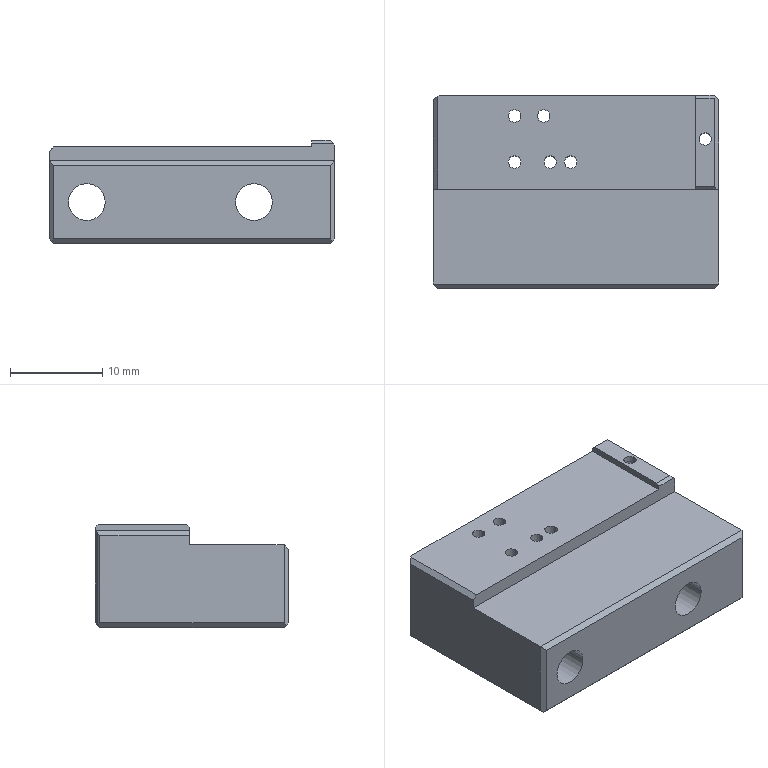Part | 1 solid | 48 faces | box 31 x 21 x 11.2 mm | volume 5475 mm3 | plane 26 | cylinder 22 | commonest cylinder face diameters 1.35 x14 4 x4 7 x4
STEP:
#1=CARTESIAN_POINT('',(2008.3,163.,-157.1));
#2=VERTEX_POINT('',#1);
#3=CARTESIAN_POINT('',(2008.3,163.,-167.3));
#4=VERTEX_POINT('',#3);
#5=CARTESIAN_POINT('',(2008.3,163.,-162.2));
#6=DIRECTION('',(0.,0.,-1.));
#7=VECTOR('',#6,1000.);
#8=LINE('',#5,#7);
#9=EDGE_CURVE('',#2,#4,#8,.T.);
#10=ORIENTED_EDGE('',*,*,#9,.F.);
#11=CARTESIAN_POINT('',(2008.3,153.3,-157.1));
#12=VERTEX_POINT('',#11);
#13=CARTESIAN_POINT('',(2008.3,158.4,-157.1));
#14=DIRECTION('',(0.,1.,0.));
#15=VECTOR('',#14,1000.);
#16=LINE('',#13,#15);
#17=EDGE_CURVE('',#12,#2,#16,.T.);
#18=ORIENTED_EDGE('',*,*,#17,.F.);
#19=CARTESIAN_POINT('',(2008.3,153.3,-158.8));
#20=VERTEX_POINT('',#19);
#21=CARTESIAN_POINT('',(2008.3,153.3,-197.47));
#22=DIRECTION('',(0.,0.,-1.));
#23=VECTOR('',#22,1000.);
#24=LINE('',#21,#23);
#25=EDGE_CURVE('',#12,#20,#24,.T.);
#26=ORIENTED_EDGE('',*,*,#25,.T.);
#27=CARTESIAN_POINT('',(2008.3,143.,-158.8));
#28=VERTEX_POINT('',#27);
#29=CARTESIAN_POINT('',(2008.3,142.5,-158.8));
#30=DIRECTION('',(0.,-1.,0.));
#31=VECTOR('',#30,1000.);
#32=LINE('',#29,#31);
#33=EDGE_CURVE('',#20,#28,#32,.T.);
#34=ORIENTED_EDGE('',*,*,#33,.T.);
#35=CARTESIAN_POINT('',(2008.3,143.,-167.3));
#36=VERTEX_POINT('',#35);
#37=CARTESIAN_POINT('',(2008.3,143.,-163.05));
#38=DIRECTION('',(0.,0.,-1.));
#39=VECTOR('',#38,1000.);
#40=LINE('',#37,#39);
#41=EDGE_CURVE('',#28,#36,#40,.T.);
#42=ORIENTED_EDGE('',*,*,#41,.T.);
#43=CARTESIAN_POINT('',(2008.3,153.,-167.3));
#44=DIRECTION('',(0.,-1.,0.));
#45=VECTOR('',#44,1000.);
#46=LINE('',#43,#45);
#47=EDGE_CURVE('',#4,#36,#46,.T.);
#48=ORIENTED_EDGE('',*,*,#47,.F.);
#49=EDGE_LOOP('',(#10,#18,#26,#34,#42,#48));
#50=FACE_BOUND('',#49,.T.);
#51=CARTESIAN_POINT('',(2008.3,142.5,-213.5));
#52=DIRECTION('',(1.,0.,0.));
#53=DIRECTION('',(0.,1.,0.));
#54=AXIS2_PLACEMENT_3D('',#51,#52,#53);
#55=PLANE('',#54);
#56=ADVANCED_FACE('',(#50),#55,.T.);
#57=CARTESIAN_POINT('',(1977.8,143.,-167.8));
#58=VERTEX_POINT('',#57);
#59=CARTESIAN_POINT('',(1977.8,163.,-167.8));
#60=VERTEX_POINT('',#59);
#61=CARTESIAN_POINT('',(1977.8,153.,-167.8));
#62=DIRECTION('',(0.,1.,0.));
#63=VECTOR('',#62,1000.);
#64=LINE('',#61,#63);
#65=EDGE_CURVE('',#58,#60,#64,.T.);
#66=ORIENTED_EDGE('',*,*,#65,.T.);
#67=CARTESIAN_POINT('',(2007.8,163.,-167.8));
#68=VERTEX_POINT('',#67);
#69=CARTESIAN_POINT('',(1992.8,163.,-167.8));
#70=DIRECTION('',(1.,0.,0.));
#71=VECTOR('',#70,1000.);
#72=LINE('',#69,#71);
#73=EDGE_CURVE('',#60,#68,#72,.T.);
#74=ORIENTED_EDGE('',*,*,#73,.T.);
#75=CARTESIAN_POINT('',(2007.8,143.,-167.8));
#76=VERTEX_POINT('',#75);
#77=CARTESIAN_POINT('',(2007.8,153.,-167.8));
#78=DIRECTION('',(0.,-1.,0.));
#79=VECTOR('',#78,1000.);
#80=LINE('',#77,#79);
#81=EDGE_CURVE('',#68,#76,#80,.T.);
#82=ORIENTED_EDGE('',*,*,#81,.T.);
#83=CARTESIAN_POINT('',(1992.8,143.,-167.8));
#84=DIRECTION('',(-1.,0.,0.));
#85=VECTOR('',#84,1000.);
#86=LINE('',#83,#85);
#87=EDGE_CURVE('',#76,#58,#86,.T.);
#88=ORIENTED_EDGE('',*,*,#87,.T.);
#89=EDGE_LOOP('',(#66,#74,#82,#88));
#90=FACE_BOUND('',#89,.T.);
#91=CARTESIAN_POINT('',(1986.795,156.238,-167.8));
#92=VERTEX_POINT('',#91);
#93=CARTESIAN_POINT('',(1985.445,156.238,-167.8));
#94=VERTEX_POINT('',#93);
#95=CARTESIAN_POINT('',(1986.12,156.238,-167.8));
#96=DIRECTION('',(0.,0.,1.));
#97=DIRECTION('',(-1.,0.,0.));
#98=AXIS2_PLACEMENT_3D('',#95,#96,#97);
#99=CIRCLE('',#98,0.675);
#100=EDGE_CURVE('',#92,#94,#99,.T.);
#101=ORIENTED_EDGE('',*,*,#100,.T.);
#102=CARTESIAN_POINT('',(1986.12,156.238,-167.8));
#103=DIRECTION('',(0.,0.,1.));
#104=DIRECTION('',(-1.,0.,0.));
#105=AXIS2_PLACEMENT_3D('',#102,#103,#104);
#106=CIRCLE('',#105,0.675);
#107=EDGE_CURVE('',#94,#92,#106,.T.);
#108=ORIENTED_EDGE('',*,*,#107,.T.);
#109=EDGE_LOOP('',(#101,#108));
#110=FACE_BOUND('',#109,.T.);
#111=CARTESIAN_POINT('',(1992.885,156.238,-167.8));
#112=VERTEX_POINT('',#111);
#113=CARTESIAN_POINT('',(1991.535,156.238,-167.8));
#114=VERTEX_POINT('',#113);
#115=CARTESIAN_POINT('',(1992.21,156.238,-167.8));
#116=DIRECTION('',(0.,0.,1.));
#117=DIRECTION('',(-1.,0.,0.));
#118=AXIS2_PLACEMENT_3D('',#115,#116,#117);
#119=CIRCLE('',#118,0.675);
#120=EDGE_CURVE('',#112,#114,#119,.T.);
#121=ORIENTED_EDGE('',*,*,#120,.T.);
#122=CARTESIAN_POINT('',(1992.21,156.238,-167.8));
#123=DIRECTION('',(0.,0.,1.));
#124=DIRECTION('',(-1.,0.,0.));
#125=AXIS2_PLACEMENT_3D('',#122,#123,#124);
#126=CIRCLE('',#125,0.675);
#127=EDGE_CURVE('',#114,#112,#126,.T.);
#128=ORIENTED_EDGE('',*,*,#127,.T.);
#129=EDGE_LOOP('',(#121,#128));
#130=FACE_BOUND('',#129,.T.);
#131=CARTESIAN_POINT('',(2007.525,158.748,-167.8));
#132=VERTEX_POINT('',#131);
#133=CARTESIAN_POINT('',(2006.175,158.748,-167.8));
#134=VERTEX_POINT('',#133);
#135=CARTESIAN_POINT('',(2006.85,158.748,-167.8));
#136=DIRECTION('',(0.,0.,-1.));
#137=DIRECTION('',(-1.,0.,0.));
#138=AXIS2_PLACEMENT_3D('',#135,#136,#137);
#139=CIRCLE('',#138,0.675);
#140=EDGE_CURVE('',#132,#134,#139,.T.);
#141=ORIENTED_EDGE('',*,*,#140,.F.);
#142=CARTESIAN_POINT('',(2006.85,158.748,-167.8));
#143=DIRECTION('',(0.,0.,-1.));
#144=DIRECTION('',(-1.,0.,0.));
#145=AXIS2_PLACEMENT_3D('',#142,#143,#144);
#146=CIRCLE('',#145,0.675);
#147=EDGE_CURVE('',#134,#132,#146,.T.);
#148=ORIENTED_EDGE('',*,*,#147,.F.);
#149=EDGE_LOOP('',(#141,#148));
#150=FACE_BOUND('',#149,.T.);
#151=CARTESIAN_POINT('',(1986.795,161.259,-167.8));
#152=VERTEX_POINT('',#151);
#153=CARTESIAN_POINT('',(1985.445,161.259,-167.8));
#154=VERTEX_POINT('',#153);
#155=CARTESIAN_POINT('',(1986.12,161.259,-167.8));
#156=DIRECTION('',(0.,0.,1.));
#157=DIRECTION('',(-1.,0.,0.));
#158=AXIS2_PLACEMENT_3D('',#155,#156,#157);
#159=CIRCLE('',#158,0.675);
#160=EDGE_CURVE('',#152,#154,#159,.T.);
#161=ORIENTED_EDGE('',*,*,#160,.T.);
#162=CARTESIAN_POINT('',(1986.12,161.259,-167.8));
#163=DIRECTION('',(0.,0.,1.));
#164=DIRECTION('',(-1.,0.,0.));
#165=AXIS2_PLACEMENT_3D('',#162,#163,#164);
#166=CIRCLE('',#165,0.675);
#167=EDGE_CURVE('',#154,#152,#166,.T.);
#168=ORIENTED_EDGE('',*,*,#167,.T.);
#169=EDGE_LOOP('',(#161,#168));
#170=FACE_BOUND('',#169,.T.);
#171=CARTESIAN_POINT('',(1989.958,161.259,-167.8));
#172=VERTEX_POINT('',#171);
#173=CARTESIAN_POINT('',(1988.608,161.259,-167.8));
#174=VERTEX_POINT('',#173);
#175=CARTESIAN_POINT('',(1989.283,161.259,-167.8));
#176=DIRECTION('',(0.,0.,1.));
#177=DIRECTION('',(-1.,0.,0.));
#178=AXIS2_PLACEMENT_3D('',#175,#176,#177);
#179=CIRCLE('',#178,0.675);
#180=EDGE_CURVE('',#172,#174,#179,.T.);
#181=ORIENTED_EDGE('',*,*,#180,.T.);
#182=CARTESIAN_POINT('',(1989.283,161.259,-167.8));
#183=DIRECTION('',(0.,0.,1.));
#184=DIRECTION('',(-1.,0.,0.));
#185=AXIS2_PLACEMENT_3D('',#182,#183,#184);
#186=CIRCLE('',#185,0.675);
#187=EDGE_CURVE('',#174,#172,#186,.T.);
#188=ORIENTED_EDGE('',*,*,#187,.T.);
#189=EDGE_LOOP('',(#181,#188));
#190=FACE_BOUND('',#189,.T.);
#191=CARTESIAN_POINT('',(1990.685,156.238,-167.8));
#192=VERTEX_POINT('',#191);
#193=CARTESIAN_POINT('',(1989.335,156.238,-167.8));
#194=VERTEX_POINT('',#193);
#195=CARTESIAN_POINT('',(1990.01,156.238,-167.8));
#196=DIRECTION('',(0.,0.,1.));
#197=DIRECTION('',(-1.,0.,0.));
#198=AXIS2_PLACEMENT_3D('',#195,#196,#197);
#199=CIRCLE('',#198,0.675);
#200=EDGE_CURVE('',#192,#194,#199,.T.);
#201=ORIENTED_EDGE('',*,*,#200,.T.);
#202=CARTESIAN_POINT('',(1990.01,156.238,-167.8));
#203=DIRECTION('',(0.,0.,1.));
#204=DIRECTION('',(-1.,0.,0.));
#205=AXIS2_PLACEMENT_3D('',#202,#203,#204);
#206=CIRCLE('',#205,0.675);
#207=EDGE_CURVE('',#194,#192,#206,.T.);
#208=ORIENTED_EDGE('',*,*,#207,.T.);
#209=EDGE_LOOP('',(#201,#208));
#210=FACE_BOUND('',#209,.T.);
#211=CARTESIAN_POINT('',(2010.,142.5,-167.8));
#212=DIRECTION('',(0.,0.,-1.));
#213=DIRECTION('',(0.,-1.,0.));
#214=AXIS2_PLACEMENT_3D('',#211,#212,#213);
#215=PLANE('',#214);
#216=ADVANCED_FACE('',(#90,#110,#130,#150,#170,#190,#210),#215,.T.);
#217=CARTESIAN_POINT('',(1977.3,163.,-157.8));
#218=VERTEX_POINT('',#217);
#219=CARTESIAN_POINT('',(1977.3,153.3,-157.8));
#220=VERTEX_POINT('',#219);
#221=CARTESIAN_POINT('',(1977.3,158.4,-157.8));
#222=DIRECTION('',(0.,-1.,0.));
#223=VECTOR('',#222,1000.);
#224=LINE('',#221,#223);
#225=EDGE_CURVE('',#218,#220,#224,.T.);
#226=ORIENTED_EDGE('',*,*,#225,.F.);
#227=CARTESIAN_POINT('',(1977.3,163.,-167.3));
#228=VERTEX_POINT('',#227);
#229=CARTESIAN_POINT('',(1977.3,163.,-162.55));
#230=DIRECTION('',(0.,0.,1.));
#231=VECTOR('',#230,1000.);
#232=LINE('',#229,#231);
#233=EDGE_CURVE('',#228,#218,#232,.T.);
#234=ORIENTED_EDGE('',*,*,#233,.F.);
#235=CARTESIAN_POINT('',(1977.3,143.,-167.3));
#236=VERTEX_POINT('',#235);
#237=CARTESIAN_POINT('',(1977.3,153.,-167.3));
#238=DIRECTION('',(0.,1.,0.));
#239=VECTOR('',#238,1000.);
#240=LINE('',#237,#239);
#241=EDGE_CURVE('',#236,#228,#240,.T.);
#242=ORIENTED_EDGE('',*,*,#241,.F.);
#243=CARTESIAN_POINT('',(1977.3,143.,-158.8));
#244=VERTEX_POINT('',#243);
#245=CARTESIAN_POINT('',(1977.3,143.,-163.05));
#246=DIRECTION('',(0.,0.,1.));
#247=VECTOR('',#246,1000.);
#248=LINE('',#245,#247);
#249=EDGE_CURVE('',#236,#244,#248,.T.);
#250=ORIENTED_EDGE('',*,*,#249,.T.);
#251=CARTESIAN_POINT('',(1977.3,153.3,-158.8));
#252=VERTEX_POINT('',#251);
#253=CARTESIAN_POINT('',(1977.3,142.5,-158.8));
#254=DIRECTION('',(0.,1.,0.));
#255=VECTOR('',#254,1000.);
#256=LINE('',#253,#255);
#257=EDGE_CURVE('',#244,#252,#256,.T.);
#258=ORIENTED_EDGE('',*,*,#257,.T.);
#259=CARTESIAN_POINT('',(1977.3,153.3,-197.47));
#260=DIRECTION('',(0.,0.,1.));
#261=VECTOR('',#260,1000.);
#262=LINE('',#259,#261);
#263=EDGE_CURVE('',#252,#220,#262,.T.);
#264=ORIENTED_EDGE('',*,*,#263,.T.);
#265=EDGE_LOOP('',(#226,#234,#242,#250,#258,#264));
#266=FACE_BOUND('',#265,.T.);
#267=CARTESIAN_POINT('',(1977.3,142.5,-205.7));
#268=DIRECTION('',(-1.,0.,0.));
#269=DIRECTION('',(0.,0.,1.));
#270=AXIS2_PLACEMENT_3D('',#267,#268,#269);
#271=PLANE('',#270);
#272=ADVANCED_FACE('',(#266),#271,.T.);
#273=CARTESIAN_POINT('',(2005.8,153.3,-156.9));
#274=VERTEX_POINT('',#273);
#275=CARTESIAN_POINT('',(2005.8,153.3,-157.3));
#276=VERTEX_POINT('',#275);
#277=CARTESIAN_POINT('',(2005.8,153.3,-197.47));
#278=DIRECTION('',(0.,0.,-1.));
#279=VECTOR('',#278,1000.);
#280=LINE('',#277,#279);
#281=EDGE_CURVE('',#274,#276,#280,.T.);
#282=ORIENTED_EDGE('',*,*,#281,.F.);
#283=CARTESIAN_POINT('',(2005.8,153.6,-156.6));
#284=VERTEX_POINT('',#283);
#285=CARTESIAN_POINT('',(2005.8,142.5,-167.7));
#286=DIRECTION('',(0.,0.7071,0.7071));
#287=VECTOR('',#286,1000.);
#288=LINE('',#285,#287);
#289=EDGE_CURVE('',#274,#284,#288,.T.);
#290=ORIENTED_EDGE('',*,*,#289,.T.);
#291=CARTESIAN_POINT('',(2005.8,163.2,-156.6));
#292=VERTEX_POINT('',#291);
#293=CARTESIAN_POINT('',(2005.8,142.5,-156.6));
#294=DIRECTION('',(0.,1.,0.));
#295=VECTOR('',#294,1000.);
#296=LINE('',#293,#295);
#297=EDGE_CURVE('',#284,#292,#296,.T.);
#298=ORIENTED_EDGE('',*,*,#297,.T.);
#299=CARTESIAN_POINT('',(2005.8,163.5,-156.9));
#300=VERTEX_POINT('',#299);
#301=CARTESIAN_POINT('',(2005.8,142.5,-135.9));
#302=DIRECTION('',(0.,-0.7071,0.7071));
#303=VECTOR('',#302,1000.);
#304=LINE('',#301,#303);
#305=EDGE_CURVE('',#300,#292,#304,.T.);
#306=ORIENTED_EDGE('',*,*,#305,.F.);
#307=CARTESIAN_POINT('',(2005.8,163.5,-157.3));
#308=VERTEX_POINT('',#307);
#309=CARTESIAN_POINT('',(2005.8,163.5,-197.47));
#310=DIRECTION('',(0.,0.,-1.));
#311=VECTOR('',#310,1000.);
#312=LINE('',#309,#311);
#313=EDGE_CURVE('',#300,#308,#312,.T.);
#314=ORIENTED_EDGE('',*,*,#313,.T.);
#315=CARTESIAN_POINT('',(2005.8,142.5,-157.3));
#316=DIRECTION('',(0.,-1.,0.));
#317=VECTOR('',#316,1000.);
#318=LINE('',#315,#317);
#319=EDGE_CURVE('',#308,#276,#318,.T.);
#320=ORIENTED_EDGE('',*,*,#319,.T.);
#321=EDGE_LOOP('',(#282,#290,#298,#306,#314,#320));
#322=FACE_BOUND('',#321,.T.);
#323=CARTESIAN_POINT('',(2005.8,142.5,-157.3));
#324=DIRECTION('',(-1.,0.,0.));
#325=DIRECTION('',(0.,0.,1.));
#326=AXIS2_PLACEMENT_3D('',#323,#324,#325);
#327=PLANE('',#326);
#328=ADVANCED_FACE('',(#322),#327,.T.);
#329=CARTESIAN_POINT('',(1986.795,161.259,-157.3));
#330=VERTEX_POINT('',#329);
#331=CARTESIAN_POINT('',(1985.445,161.259,-157.3));
#332=VERTEX_POINT('',#331);
#333=CARTESIAN_POINT('',(1986.12,161.259,-157.3));
#334=DIRECTION('',(0.,0.,1.));
#335=DIRECTION('',(-1.,0.,0.));
#336=AXIS2_PLACEMENT_3D('',#333,#334,#335);
#337=CIRCLE('',#336,0.675);
#338=EDGE_CURVE('',#330,#332,#337,.T.);
#339=ORIENTED_EDGE('',*,*,#338,.T.);
#340=CARTESIAN_POINT('',(1985.445,161.259,-157.3));
#341=DIRECTION('',(0.,0.,1.));
#342=VECTOR('',#341,1000.);
#343=LINE('',#340,#342);
#344=EDGE_CURVE('',#332,#154,#343,.F.);
#345=ORIENTED_EDGE('',*,*,#344,.T.);
#346=ORIENTED_EDGE('',*,*,#160,.F.);
#347=CARTESIAN_POINT('',(1986.795,161.259,-157.3));
#348=DIRECTION('',(0.,0.,1.));
#349=VECTOR('',#348,1000.);
#350=LINE('',#347,#349);
#351=EDGE_CURVE('',#330,#152,#350,.F.);
#352=ORIENTED_EDGE('',*,*,#351,.F.);
#353=EDGE_LOOP('',(#339,#345,#346,#352));
#354=FACE_BOUND('',#353,.T.);
#355=CARTESIAN_POINT('',(1986.12,161.259,-157.3));
#356=DIRECTION('',(0.,0.,1.));
#357=DIRECTION('',(-1.,0.,0.));
#358=AXIS2_PLACEMENT_3D('',#355,#356,#357);
#359=CYLINDRICAL_SURFACE('',#358,0.675);
#360=ADVANCED_FACE('',(#354),#359,.F.);
#361=CARTESIAN_POINT('',(1989.958,161.259,-157.3));
#362=VERTEX_POINT('',#361);
#363=CARTESIAN_POINT('',(1988.608,161.259,-157.3));
#364=VERTEX_POINT('',#363);
#365=CARTESIAN_POINT('',(1989.283,161.259,-157.3));
#366=DIRECTION('',(0.,0.,1.));
#367=DIRECTION('',(-1.,0.,0.));
#368=AXIS2_PLACEMENT_3D('',#365,#366,#367);
#369=CIRCLE('',#368,0.675);
#370=EDGE_CURVE('',#362,#364,#369,.T.);
#371=ORIENTED_EDGE('',*,*,#370,.T.);
#372=CARTESIAN_POINT('',(1988.608,161.259,-157.3));
#373=DIRECTION('',(0.,0.,1.));
#374=VECTOR('',#373,1000.);
#375=LINE('',#372,#374);
#376=EDGE_CURVE('',#364,#174,#375,.F.);
#377=ORIENTED_EDGE('',*,*,#376,.T.);
#378=ORIENTED_EDGE('',*,*,#180,.F.);
#379=CARTESIAN_POINT('',(1989.958,161.259,-157.3));
#380=DIRECTION('',(0.,0.,1.));
#381=VECTOR('',#380,1000.);
#382=LINE('',#379,#381);
#383=EDGE_CURVE('',#362,#172,#382,.F.);
#384=ORIENTED_EDGE('',*,*,#383,.F.);
#385=EDGE_LOOP('',(#371,#377,#378,#384));
#386=FACE_BOUND('',#385,.T.);
#387=CARTESIAN_POINT('',(1989.283,161.259,-157.3));
#388=DIRECTION('',(0.,0.,1.));
#389=DIRECTION('',(-1.,0.,0.));
#390=AXIS2_PLACEMENT_3D('',#387,#388,#389);
#391=CYLINDRICAL_SURFACE('',#390,0.675);
#392=ADVANCED_FACE('',(#386),#391,.F.);
#393=CARTESIAN_POINT('',(1990.685,156.238,-157.3));
#394=VERTEX_POINT('',#393);
#395=CARTESIAN_POINT('',(1989.335,156.238,-157.3));
#396=VERTEX_POINT('',#395);
#397=CARTESIAN_POINT('',(1990.01,156.238,-157.3));
#398=DIRECTION('',(0.,0.,1.));
#399=DIRECTION('',(-1.,0.,0.));
#400=AXIS2_PLACEMENT_3D('',#397,#398,#399);
#401=CIRCLE('',#400,0.675);
#402=EDGE_CURVE('',#394,#396,#401,.T.);
#403=ORIENTED_EDGE('',*,*,#402,.T.);
#404=CARTESIAN_POINT('',(1989.335,156.238,-157.3));
#405=DIRECTION('',(0.,0.,1.));
#406=VECTOR('',#405,1000.);
#407=LINE('',#404,#406);
#408=EDGE_CURVE('',#396,#194,#407,.F.);
#409=ORIENTED_EDGE('',*,*,#408,.T.);
#410=ORIENTED_EDGE('',*,*,#200,.F.);
#411=CARTESIAN_POINT('',(1990.685,156.238,-157.3));
#412=DIRECTION('',(0.,0.,1.));
#413=VECTOR('',#412,1000.);
#414=LINE('',#411,#413);
#415=EDGE_CURVE('',#394,#192,#414,.F.);
#416=ORIENTED_EDGE('',*,*,#415,.F.);
#417=EDGE_LOOP('',(#403,#409,#410,#416));
#418=FACE_BOUND('',#417,.T.);
#419=CARTESIAN_POINT('',(1990.01,156.238,-157.3));
#420=DIRECTION('',(0.,0.,1.));
#421=DIRECTION('',(-1.,0.,0.));
#422=AXIS2_PLACEMENT_3D('',#419,#420,#421);
#423=CYLINDRICAL_SURFACE('',#422,0.675);
#424=ADVANCED_FACE('',(#418),#423,.F.);
#425=CARTESIAN_POINT('',(1986.795,156.238,-157.3));
#426=VERTEX_POINT('',#425);
#427=CARTESIAN_POINT('',(1985.445,156.238,-157.3));
#428=VERTEX_POINT('',#427);
#429=CARTESIAN_POINT('',(1986.12,156.238,-157.3));
#430=DIRECTION('',(0.,0.,1.));
#431=DIRECTION('',(-1.,0.,0.));
#432=AXIS2_PLACEMENT_3D('',#429,#430,#431);
#433=CIRCLE('',#432,0.675);
#434=EDGE_CURVE('',#426,#428,#433,.T.);
#435=ORIENTED_EDGE('',*,*,#434,.T.);
#436=CARTESIAN_POINT('',(1985.445,156.238,-157.3));
#437=DIRECTION('',(0.,0.,1.));
#438=VECTOR('',#437,1000.);
#439=LINE('',#436,#438);
#440=EDGE_CURVE('',#428,#94,#439,.F.);
#441=ORIENTED_EDGE('',*,*,#440,.T.);
#442=ORIENTED_EDGE('',*,*,#100,.F.);
#443=CARTESIAN_POINT('',(1986.795,156.238,-157.3));
#444=DIRECTION('',(0.,0.,1.));
#445=VECTOR('',#444,1000.);
#446=LINE('',#443,#445);
#447=EDGE_CURVE('',#426,#92,#446,.F.);
#448=ORIENTED_EDGE('',*,*,#447,.F.);
#449=EDGE_LOOP('',(#435,#441,#442,#448));
#450=FACE_BOUND('',#449,.T.);
#451=CARTESIAN_POINT('',(1986.12,156.238,-157.3));
#452=DIRECTION('',(0.,0.,1.));
#453=DIRECTION('',(-1.,0.,0.));
#454=AXIS2_PLACEMENT_3D('',#451,#452,#453);
#455=CYLINDRICAL_SURFACE('',#454,0.675);
#456=ADVANCED_FACE('',(#450),#455,.F.);
#457=CARTESIAN_POINT('',(1992.885,156.238,-157.3));
#458=VERTEX_POINT('',#457);
#459=CARTESIAN_POINT('',(1991.535,156.238,-157.3));
#460=VERTEX_POINT('',#459);
#461=CARTESIAN_POINT('',(1992.21,156.238,-157.3));
#462=DIRECTION('',(0.,0.,1.));
#463=DIRECTION('',(-1.,0.,0.));
#464=AXIS2_PLACEMENT_3D('',#461,#462,#463);
#465=CIRCLE('',#464,0.675);
#466=EDGE_CURVE('',#458,#460,#465,.T.);
#467=ORIENTED_EDGE('',*,*,#466,.T.);
#468=CARTESIAN_POINT('',(1991.535,156.238,-157.3));
#469=DIRECTION('',(0.,0.,1.));
#470=VECTOR('',#469,1000.);
#471=LINE('',#468,#470);
#472=EDGE_CURVE('',#460,#114,#471,.F.);
#473=ORIENTED_EDGE('',*,*,#472,.T.);
#474=ORIENTED_EDGE('',*,*,#120,.F.);
#475=CARTESIAN_POINT('',(1992.885,156.238,-157.3));
#476=DIRECTION('',(0.,0.,1.));
#477=VECTOR('',#476,1000.);
#478=LINE('',#475,#477);
#479=EDGE_CURVE('',#458,#112,#478,.F.);
#480=ORIENTED_EDGE('',*,*,#479,.F.);
#481=EDGE_LOOP('',(#467,#473,#474,#480));
#482=FACE_BOUND('',#481,.T.);
#483=CARTESIAN_POINT('',(1992.21,156.238,-157.3));
#484=DIRECTION('',(0.,0.,1.));
#485=DIRECTION('',(-1.,0.,0.));
#486=AXIS2_PLACEMENT_3D('',#483,#484,#485);
#487=CYLINDRICAL_SURFACE('',#486,0.675);
#488=ADVANCED_FACE('',(#482),#487,.F.);
#489=CARTESIAN_POINT('',(2007.525,158.748,-157.3));
#490=VERTEX_POINT('',#489);
#491=CARTESIAN_POINT('',(2006.175,158.748,-157.3));
#492=VERTEX_POINT('',#491);
#493=CARTESIAN_POINT('',(2006.85,158.748,-157.3));
#494=DIRECTION('',(0.,0.,-1.));
#495=DIRECTION('',(-1.,0.,0.));
#496=AXIS2_PLACEMENT_3D('',#493,#494,#495);
#497=CIRCLE('',#496,0.675);
#498=EDGE_CURVE('',#490,#492,#497,.T.);
#499=ORIENTED_EDGE('',*,*,#498,.F.);
#500=CARTESIAN_POINT('',(2007.525,158.748,-157.3));
#501=DIRECTION('',(0.,0.,1.));
#502=VECTOR('',#501,1000.);
#503=LINE('',#500,#502);
#504=EDGE_CURVE('',#490,#132,#503,.F.);
#505=ORIENTED_EDGE('',*,*,#504,.T.);
#506=ORIENTED_EDGE('',*,*,#140,.T.);
#507=CARTESIAN_POINT('',(2006.175,158.748,-157.3));
#508=DIRECTION('',(0.,0.,1.));
#509=VECTOR('',#508,1000.);
#510=LINE('',#507,#509);
#511=EDGE_CURVE('',#492,#134,#510,.F.);
#512=ORIENTED_EDGE('',*,*,#511,.F.);
#513=EDGE_LOOP('',(#499,#505,#506,#512));
#514=FACE_BOUND('',#513,.T.);
#515=CARTESIAN_POINT('',(2006.85,158.748,-157.3));
#516=DIRECTION('',(0.,0.,1.));
#517=DIRECTION('',(-1.,0.,0.));
#518=AXIS2_PLACEMENT_3D('',#515,#516,#517);
#519=CYLINDRICAL_SURFACE('',#518,0.675);
#520=ADVANCED_FACE('',(#514),#519,.F.);
#521=CARTESIAN_POINT('',(1977.8,153.3,-157.3));
#522=VERTEX_POINT('',#521);
#523=CARTESIAN_POINT('',(1983.678,153.3,-157.3));
#524=DIRECTION('',(-1.,0.,0.));
#525=VECTOR('',#524,1000.);
#526=LINE('',#523,#525);
#527=EDGE_CURVE('',#276,#522,#526,.T.);
#528=ORIENTED_EDGE('',*,*,#527,.F.);
#529=ORIENTED_EDGE('',*,*,#319,.F.);
#530=CARTESIAN_POINT('',(1978.1,163.5,-157.3));
#531=VERTEX_POINT('',#530);
#532=CARTESIAN_POINT('',(1983.678,163.5,-157.3));
#533=DIRECTION('',(-1.,0.,0.));
#534=VECTOR('',#533,1000.);
#535=LINE('',#532,#534);
#536=EDGE_CURVE('',#308,#531,#535,.T.);
#537=ORIENTED_EDGE('',*,*,#536,.T.);
#538=CARTESIAN_POINT('',(1977.8,163.376,-157.3));
#539=VERTEX_POINT('',#538);
#540=CARTESIAN_POINT('',(1983.678,165.81,-157.3));
#541=DIRECTION('',(0.9239,0.3827,0.));
#542=VECTOR('',#541,1000.);
#543=LINE('',#540,#542);
#544=EDGE_CURVE('',#539,#531,#543,.T.);
#545=ORIENTED_EDGE('',*,*,#544,.F.);
#546=CARTESIAN_POINT('',(1977.8,158.4,-157.3));
#547=DIRECTION('',(0.,-1.,0.));
#548=VECTOR('',#547,1000.);
#549=LINE('',#546,#548);
#550=EDGE_CURVE('',#539,#522,#549,.T.);
#551=ORIENTED_EDGE('',*,*,#550,.T.);
#552=EDGE_LOOP('',(#528,#529,#537,#545,#551));
#553=FACE_BOUND('',#552,.T.);
#554=ORIENTED_EDGE('',*,*,#402,.F.);
#555=CARTESIAN_POINT('',(1990.01,156.238,-157.3));
#556=DIRECTION('',(0.,0.,1.));
#557=DIRECTION('',(-1.,0.,0.));
#558=AXIS2_PLACEMENT_3D('',#555,#556,#557);
#559=CIRCLE('',#558,0.675);
#560=EDGE_CURVE('',#396,#394,#559,.T.);
#561=ORIENTED_EDGE('',*,*,#560,.F.);
#562=EDGE_LOOP('',(#554,#561));
#563=FACE_BOUND('',#562,.T.);
#564=ORIENTED_EDGE('',*,*,#434,.F.);
#565=CARTESIAN_POINT('',(1986.12,156.238,-157.3));
#566=DIRECTION('',(0.,0.,1.));
#567=DIRECTION('',(-1.,0.,0.));
#568=AXIS2_PLACEMENT_3D('',#565,#566,#567);
#569=CIRCLE('',#568,0.675);
#570=EDGE_CURVE('',#428,#426,#569,.T.);
#571=ORIENTED_EDGE('',*,*,#570,.F.);
#572=EDGE_LOOP('',(#564,#571));
#573=FACE_BOUND('',#572,.T.);
#574=ORIENTED_EDGE('',*,*,#466,.F.);
#575=CARTESIAN_POINT('',(1992.21,156.238,-157.3));
#576=DIRECTION('',(0.,0.,1.));
#577=DIRECTION('',(-1.,0.,0.));
#578=AXIS2_PLACEMENT_3D('',#575,#576,#577);
#579=CIRCLE('',#578,0.675);
#580=EDGE_CURVE('',#460,#458,#579,.T.);
#581=ORIENTED_EDGE('',*,*,#580,.F.);
#582=EDGE_LOOP('',(#574,#581));
#583=FACE_BOUND('',#582,.T.);
#584=ORIENTED_EDGE('',*,*,#338,.F.);
#585=CARTESIAN_POINT('',(1986.12,161.259,-157.3));
#586=DIRECTION('',(0.,0.,1.));
#587=DIRECTION('',(-1.,0.,0.));
#588=AXIS2_PLACEMENT_3D('',#585,#586,#587);
#589=CIRCLE('',#588,0.675);
#590=EDGE_CURVE('',#332,#330,#589,.T.);
#591=ORIENTED_EDGE('',*,*,#590,.F.);
#592=EDGE_LOOP('',(#584,#591));
#593=FACE_BOUND('',#592,.T.);
#594=ORIENTED_EDGE('',*,*,#370,.F.);
#595=CARTESIAN_POINT('',(1989.283,161.259,-157.3));
#596=DIRECTION('',(0.,0.,1.));
#597=DIRECTION('',(-1.,0.,0.));
#598=AXIS2_PLACEMENT_3D('',#595,#596,#597);
#599=CIRCLE('',#598,0.675);
#600=EDGE_CURVE('',#364,#362,#599,.T.);
#601=ORIENTED_EDGE('',*,*,#600,.F.);
#602=EDGE_LOOP('',(#594,#601));
#603=FACE_BOUND('',#602,.T.);
#604=CARTESIAN_POINT('',(2010.3,142.5,-157.3));
#605=DIRECTION('',(0.,0.,1.));
#606=DIRECTION('',(1.,0.,0.));
#607=AXIS2_PLACEMENT_3D('',#604,#605,#606);
#608=PLANE('',#607);
#609=ADVANCED_FACE('',(#553,#563,#573,#583,#593,#603),#608,.T.);
#610=CARTESIAN_POINT('',(2007.8,153.6,-156.6));
#611=VERTEX_POINT('',#610);
#612=CARTESIAN_POINT('',(2006.8,153.6,-156.6));
#613=DIRECTION('',(-1.,0.,0.));
#614=VECTOR('',#613,1000.);
#615=LINE('',#612,#614);
#616=EDGE_CURVE('',#611,#284,#615,.T.);
#617=ORIENTED_EDGE('',*,*,#616,.F.);
#618=CARTESIAN_POINT('',(2007.8,163.2,-156.6));
#619=VERTEX_POINT('',#618);
#620=CARTESIAN_POINT('',(2007.8,158.4,-156.6));
#621=DIRECTION('',(0.,1.,0.));
#622=VECTOR('',#621,1000.);
#623=LINE('',#620,#622);
#624=EDGE_CURVE('',#611,#619,#623,.T.);
#625=ORIENTED_EDGE('',*,*,#624,.T.);
#626=CARTESIAN_POINT('',(2006.8,163.2,-156.6));
#627=DIRECTION('',(-1.,0.,0.));
#628=VECTOR('',#627,1000.);
#629=LINE('',#626,#628);
#630=EDGE_CURVE('',#619,#292,#629,.T.);
#631=ORIENTED_EDGE('',*,*,#630,.T.);
#632=ORIENTED_EDGE('',*,*,#297,.F.);
#633=EDGE_LOOP('',(#617,#625,#631,#632));
#634=FACE_BOUND('',#633,.T.);
#635=CARTESIAN_POINT('',(2007.525,158.748,-156.6));
#636=VERTEX_POINT('',#635);
#637=CARTESIAN_POINT('',(2006.175,158.748,-156.6));
#638=VERTEX_POINT('',#637);
#639=CARTESIAN_POINT('',(2006.85,158.748,-156.6));
#640=DIRECTION('',(0.,0.,-1.));
#641=DIRECTION('',(-1.,0.,0.));
#642=AXIS2_PLACEMENT_3D('',#639,#640,#641);
#643=CIRCLE('',#642,0.675);
#644=EDGE_CURVE('',#636,#638,#643,.T.);
#645=ORIENTED_EDGE('',*,*,#644,.T.);
#646=CARTESIAN_POINT('',(2006.85,158.748,-156.6));
#647=DIRECTION('',(0.,0.,-1.));
#648=DIRECTION('',(-1.,0.,0.));
#649=AXIS2_PLACEMENT_3D('',#646,#647,#648);
#650=CIRCLE('',#649,0.675);
#651=EDGE_CURVE('',#638,#636,#650,.T.);
#652=ORIENTED_EDGE('',*,*,#651,.T.);
#653=EDGE_LOOP('',(#645,#652));
#654=FACE_BOUND('',#653,.T.);
#655=CARTESIAN_POINT('',(2008.974,161.53,-156.6));
#656=DIRECTION('',(0.,0.,1.));
#657=DIRECTION('',(1.,0.,0.));
#658=AXIS2_PLACEMENT_3D('',#655,#656,#657);
#659=PLANE('',#658);
#660=ADVANCED_FACE('',(#634,#654),#659,.T.);
#661=ORIENTED_EDGE('',*,*,#624,.F.);
#662=CARTESIAN_POINT('',(2008.1,153.3,-156.9));
#663=VERTEX_POINT('',#662);
#664=CARTESIAN_POINT('',(2018.9,142.5,-167.7));
#665=DIRECTION('',(0.5774,-0.5774,-0.5774));
#666=VECTOR('',#665,1000.);
#667=LINE('',#664,#666);
#668=EDGE_CURVE('',#611,#663,#667,.T.);
#669=ORIENTED_EDGE('',*,*,#668,.T.);
#670=CARTESIAN_POINT('',(2048.67,153.3,-197.47));
#671=DIRECTION('',(-0.7071,0.,0.7071));
#672=VECTOR('',#671,1000.);
#673=LINE('',#670,#672);
#674=EDGE_CURVE('',#12,#663,#673,.T.);
#675=ORIENTED_EDGE('',*,*,#674,.F.);
#676=ORIENTED_EDGE('',*,*,#17,.T.);
#677=CARTESIAN_POINT('',(2007.95,163.35,-156.75));
#678=VERTEX_POINT('',#677);
#679=CARTESIAN_POINT('',(2028.8,142.5,-177.6));
#680=DIRECTION('',(-0.5774,0.5774,0.5774));
#681=VECTOR('',#680,1000.);
#682=LINE('',#679,#681);
#683=EDGE_CURVE('',#2,#678,#682,.T.);
#684=ORIENTED_EDGE('',*,*,#683,.T.);
#685=CARTESIAN_POINT('',(1987.1,142.5,-135.9));
#686=DIRECTION('',(0.5774,0.5774,-0.5774));
#687=VECTOR('',#686,1000.);
#688=LINE('',#685,#687);
#689=EDGE_CURVE('',#619,#678,#688,.T.);
#690=ORIENTED_EDGE('',*,*,#689,.F.);
#691=EDGE_LOOP('',(#661,#669,#675,#676,#684,#690));
#692=FACE_BOUND('',#691,.T.);
#693=CARTESIAN_POINT('',(2008.05,158.4,-156.85));
#694=DIRECTION('',(0.7071,0.,0.7071));
#695=DIRECTION('',(0.,-1.,0.));
#696=AXIS2_PLACEMENT_3D('',#693,#694,#695);
#697=PLANE('',#696);
#698=ADVANCED_FACE('',(#692),#697,.T.);
#699=ORIENTED_EDGE('',*,*,#25,.F.);
#700=ORIENTED_EDGE('',*,*,#674,.T.);
#701=CARTESIAN_POINT('',(2006.8,153.3,-156.9));
#702=DIRECTION('',(-1.,0.,0.));
#703=VECTOR('',#702,1000.);
#704=LINE('',#701,#703);
#705=EDGE_CURVE('',#663,#274,#704,.T.);
#706=ORIENTED_EDGE('',*,*,#705,.T.);
#707=ORIENTED_EDGE('',*,*,#281,.T.);
#708=ORIENTED_EDGE('',*,*,#527,.T.);
#709=CARTESIAN_POINT('',(1937.63,153.3,-197.47));
#710=DIRECTION('',(0.7071,0.,0.7071));
#711=VECTOR('',#710,1000.);
#712=LINE('',#709,#711);
#713=EDGE_CURVE('',#220,#522,#712,.T.);
#714=ORIENTED_EDGE('',*,*,#713,.F.);
#715=ORIENTED_EDGE('',*,*,#263,.F.);
#716=CARTESIAN_POINT('',(1983.678,153.3,-158.8));
#717=DIRECTION('',(-1.,0.,0.));
#718=VECTOR('',#717,1000.);
#719=LINE('',#716,#718);
#720=EDGE_CURVE('',#20,#252,#719,.T.);
#721=ORIENTED_EDGE('',*,*,#720,.F.);
#722=EDGE_LOOP('',(#699,#700,#706,#707,#708,#714,#715,#721));
#723=FACE_BOUND('',#722,.T.);
#724=CARTESIAN_POINT('',(1975.1,153.3,-156.6));
#725=DIRECTION('',(0.,1.,0.));
#726=DIRECTION('',(1.,0.,0.));
#727=AXIS2_PLACEMENT_3D('',#724,#725,#726);
#728=PLANE('',#727);
#729=ADVANCED_FACE('',(#723),#728,.F.);
#730=ORIENTED_EDGE('',*,*,#257,.F.);
#731=CARTESIAN_POINT('',(1992.8,143.,-158.8));
#732=DIRECTION('',(-1.,0.,0.));
#733=VECTOR('',#732,1000.);
#734=LINE('',#731,#733);
#735=EDGE_CURVE('',#28,#244,#734,.T.);
#736=ORIENTED_EDGE('',*,*,#735,.F.);
#737=ORIENTED_EDGE('',*,*,#33,.F.);
#738=ORIENTED_EDGE('',*,*,#720,.T.);
#739=EDGE_LOOP('',(#730,#736,#737,#738));
#740=FACE_BOUND('',#739,.T.);
#741=CARTESIAN_POINT('',(1975.1,153.3,-158.8));
#742=DIRECTION('',(0.,0.,-1.));
#743=DIRECTION('',(0.,-1.,0.));
#744=AXIS2_PLACEMENT_3D('',#741,#742,#743);
#745=PLANE('',#744);
#746=ADVANCED_FACE('',(#740),#745,.F.);
#747=ORIENTED_EDGE('',*,*,#47,.T.);
#748=CARTESIAN_POINT('',(2008.05,142.75,-167.55));
#749=VERTEX_POINT('',#748);
#750=CARTESIAN_POINT('',(2007.8,142.5,-167.8));
#751=DIRECTION('',(0.5774,0.5774,0.5774));
#752=VECTOR('',#751,1000.);
#753=LINE('',#750,#752);
#754=EDGE_CURVE('',#749,#36,#753,.T.);
#755=ORIENTED_EDGE('',*,*,#754,.F.);
#756=CARTESIAN_POINT('',(1983.678,167.122,-191.922));
#757=DIRECTION('',(0.5774,-0.5774,0.5774));
#758=VECTOR('',#757,1000.);
#759=LINE('',#756,#758);
#760=EDGE_CURVE('',#76,#749,#759,.T.);
#761=ORIENTED_EDGE('',*,*,#760,.F.);
#762=ORIENTED_EDGE('',*,*,#81,.F.);
#763=CARTESIAN_POINT('',(2008.05,163.25,-167.55));
#764=VERTEX_POINT('',#763);
#765=CARTESIAN_POINT('',(1983.678,138.878,-191.922));
#766=DIRECTION('',(0.5774,0.5774,0.5774));
#767=VECTOR('',#766,1000.);
#768=LINE('',#765,#767);
#769=EDGE_CURVE('',#68,#764,#768,.T.);
#770=ORIENTED_EDGE('',*,*,#769,.T.);
#771=CARTESIAN_POINT('',(2028.8,142.5,-146.8));
#772=DIRECTION('',(0.5774,-0.5774,0.5774));
#773=VECTOR('',#772,1000.);
#774=LINE('',#771,#773);
#775=EDGE_CURVE('',#764,#4,#774,.T.);
#776=ORIENTED_EDGE('',*,*,#775,.T.);
#777=EDGE_LOOP('',(#747,#755,#761,#762,#770,#776));
#778=FACE_BOUND('',#777,.T.);
#779=CARTESIAN_POINT('',(2008.05,153.,-167.55));
#780=DIRECTION('',(-0.7071,0.,0.7071));
#781=DIRECTION('',(0.,1.,0.));
#782=AXIS2_PLACEMENT_3D('',#779,#780,#781);
#783=PLANE('',#782);
#784=ADVANCED_FACE('',(#778),#783,.F.);
#785=ORIENTED_EDGE('',*,*,#9,.T.);
#786=ORIENTED_EDGE('',*,*,#775,.F.);
#787=CARTESIAN_POINT('',(2007.8,163.5,-167.3));
#788=VERTEX_POINT('',#787);
#789=CARTESIAN_POINT('',(2028.8,142.5,-188.3));
#790=DIRECTION('',(-0.5774,0.5774,0.5774));
#791=VECTOR('',#790,1000.);
#792=LINE('',#789,#791);
#793=EDGE_CURVE('',#764,#788,#792,.T.);
#794=ORIENTED_EDGE('',*,*,#793,.T.);
#795=CARTESIAN_POINT('',(2007.8,163.5,-156.9));
#796=VERTEX_POINT('',#795);
#797=CARTESIAN_POINT('',(2007.8,163.5,-162.2));
#798=DIRECTION('',(0.,0.,-1.));
#799=VECTOR('',#798,1000.);
#800=LINE('',#797,#799);
#801=EDGE_CURVE('',#796,#788,#800,.T.);
#802=ORIENTED_EDGE('',*,*,#801,.F.);
#803=CARTESIAN_POINT('',(2028.8,142.5,-135.9));
#804=DIRECTION('',(0.5774,-0.5774,0.5774));
#805=VECTOR('',#804,1000.);
#806=LINE('',#803,#805);
#807=EDGE_CURVE('',#796,#678,#806,.T.);
#808=ORIENTED_EDGE('',*,*,#807,.T.);
#809=ORIENTED_EDGE('',*,*,#683,.F.);
#810=EDGE_LOOP('',(#785,#786,#794,#802,#808,#809));
#811=FACE_BOUND('',#810,.T.);
#812=CARTESIAN_POINT('',(2008.05,163.25,-162.2));
#813=DIRECTION('',(-0.7071,-0.7071,0.));
#814=DIRECTION('',(-0.7071,0.7071,0.));
#815=AXIS2_PLACEMENT_3D('',#812,#813,#814);
#816=PLANE('',#815);
#817=ADVANCED_FACE('',(#811),#816,.F.);
#818=ORIENTED_EDGE('',*,*,#65,.F.);
#819=CARTESIAN_POINT('',(1977.55,142.75,-167.55));
#820=VERTEX_POINT('',#819);
#821=CARTESIAN_POINT('',(1977.3,142.5,-167.3));
#822=DIRECTION('',(-0.5774,-0.5774,0.5774));
#823=VECTOR('',#822,1000.);
#824=LINE('',#821,#823);
#825=EDGE_CURVE('',#58,#820,#824,.T.);
#826=ORIENTED_EDGE('',*,*,#825,.T.);
#827=CARTESIAN_POINT('',(2007.47,112.83,-197.47));
#828=DIRECTION('',(-0.5774,0.5774,0.5774));
#829=VECTOR('',#828,1000.);
#830=LINE('',#827,#829);
#831=EDGE_CURVE('',#820,#236,#830,.T.);
#832=ORIENTED_EDGE('',*,*,#831,.T.);
#833=ORIENTED_EDGE('',*,*,#241,.T.);
#834=CARTESIAN_POINT('',(1977.55,163.25,-167.55));
#835=VERTEX_POINT('',#834);
#836=CARTESIAN_POINT('',(2007.47,193.17,-197.47));
#837=DIRECTION('',(-0.5774,-0.5774,0.5774));
#838=VECTOR('',#837,1000.);
#839=LINE('',#836,#838);
#840=EDGE_CURVE('',#835,#228,#839,.T.);
#841=ORIENTED_EDGE('',*,*,#840,.F.);
#842=CARTESIAN_POINT('',(1998.3,142.5,-188.3));
#843=DIRECTION('',(0.5774,-0.5774,-0.5774));
#844=VECTOR('',#843,1000.);
#845=LINE('',#842,#844);
#846=EDGE_CURVE('',#835,#60,#845,.T.);
#847=ORIENTED_EDGE('',*,*,#846,.T.);
#848=EDGE_LOOP('',(#818,#826,#832,#833,#841,#847));
#849=FACE_BOUND('',#848,.T.);
#850=CARTESIAN_POINT('',(1977.55,153.,-167.55));
#851=DIRECTION('',(-0.7071,0.,-0.7071));
#852=DIRECTION('',(-0.7071,0.,0.7071));
#853=AXIS2_PLACEMENT_3D('',#850,#851,#852);
#854=PLANE('',#853);
#855=ADVANCED_FACE('',(#849),#854,.T.);
#856=ORIENTED_EDGE('',*,*,#225,.T.);
#857=ORIENTED_EDGE('',*,*,#713,.T.);
#858=ORIENTED_EDGE('',*,*,#550,.F.);
#859=CARTESIAN_POINT('',(1977.588,163.288,-157.512));
#860=VERTEX_POINT('',#859);
#861=CARTESIAN_POINT('',(1937.63,146.737,-197.47));
#862=DIRECTION('',(-0.6786,-0.2811,-0.6786));
#863=VECTOR('',#862,1000.);
#864=LINE('',#861,#863);
#865=EDGE_CURVE('',#539,#860,#864,.T.);
#866=ORIENTED_EDGE('',*,*,#865,.T.);
#867=CARTESIAN_POINT('',(1956.8,142.5,-178.3));
#868=DIRECTION('',(-0.5774,-0.5774,-0.5774));
#869=VECTOR('',#868,1000.);
#870=LINE('',#867,#869);
#871=EDGE_CURVE('',#860,#218,#870,.T.);
#872=ORIENTED_EDGE('',*,*,#871,.T.);
#873=EDGE_LOOP('',(#856,#857,#858,#866,#872));
#874=FACE_BOUND('',#873,.T.);
#875=CARTESIAN_POINT('',(1977.55,158.4,-157.55));
#876=DIRECTION('',(0.7071,0.,-0.7071));
#877=DIRECTION('',(0.,-1.,0.));
#878=AXIS2_PLACEMENT_3D('',#875,#876,#877);
#879=PLANE('',#878);
#880=ADVANCED_FACE('',(#874),#879,.F.);
#881=ORIENTED_EDGE('',*,*,#644,.F.);
#882=CARTESIAN_POINT('',(2007.525,158.748,-155.48));
#883=DIRECTION('',(0.,0.,-1.));
#884=VECTOR('',#883,1000.);
#885=LINE('',#882,#884);
#886=EDGE_CURVE('',#490,#636,#885,.F.);
#887=ORIENTED_EDGE('',*,*,#886,.F.);
#888=ORIENTED_EDGE('',*,*,#498,.T.);
#889=CARTESIAN_POINT('',(2006.175,158.748,-155.48));
#890=DIRECTION('',(0.,0.,-1.));
#891=VECTOR('',#890,1000.);
#892=LINE('',#889,#891);
#893=EDGE_CURVE('',#492,#638,#892,.F.);
#894=ORIENTED_EDGE('',*,*,#893,.T.);
#895=EDGE_LOOP('',(#881,#887,#888,#894));
#896=FACE_BOUND('',#895,.T.);
#897=CARTESIAN_POINT('',(2006.85,158.748,-155.48));
#898=DIRECTION('',(0.,0.,-1.));
#899=DIRECTION('',(-1.,0.,0.));
#900=AXIS2_PLACEMENT_3D('',#897,#898,#899);
#901=CYLINDRICAL_SURFACE('',#900,0.675);
#902=ADVANCED_FACE('',(#896),#901,.F.);
#903=ORIENTED_EDGE('',*,*,#630,.F.);
#904=ORIENTED_EDGE('',*,*,#689,.T.);
#905=ORIENTED_EDGE('',*,*,#807,.F.);
#906=CARTESIAN_POINT('',(2006.8,163.5,-156.9));
#907=DIRECTION('',(-1.,0.,0.));
#908=VECTOR('',#907,1000.);
#909=LINE('',#906,#908);
#910=EDGE_CURVE('',#796,#300,#909,.T.);
#911=ORIENTED_EDGE('',*,*,#910,.T.);
#912=ORIENTED_EDGE('',*,*,#305,.T.);
#913=EDGE_LOOP('',(#903,#904,#905,#911,#912));
#914=FACE_BOUND('',#913,.T.);
#915=CARTESIAN_POINT('',(2006.8,163.35,-156.75));
#916=DIRECTION('',(0.,0.7071,0.7071));
#917=DIRECTION('',(1.,0.,0.));
#918=AXIS2_PLACEMENT_3D('',#915,#916,#917);
#919=PLANE('',#918);
#920=ADVANCED_FACE('',(#914),#919,.T.);
#921=ORIENTED_EDGE('',*,*,#616,.T.);
#922=ORIENTED_EDGE('',*,*,#289,.F.);
#923=ORIENTED_EDGE('',*,*,#705,.F.);
#924=ORIENTED_EDGE('',*,*,#668,.F.);
#925=EDGE_LOOP('',(#921,#922,#923,#924));
#926=FACE_BOUND('',#925,.T.);
#927=CARTESIAN_POINT('',(2006.8,153.45,-156.75));
#928=DIRECTION('',(0.,0.7071,-0.7071));
#929=DIRECTION('',(-1.,0.,0.));
#930=AXIS2_PLACEMENT_3D('',#927,#928,#929);
#931=PLANE('',#930);
#932=ADVANCED_FACE('',(#926),#931,.F.);
#933=ORIENTED_EDGE('',*,*,#893,.F.);
#934=CARTESIAN_POINT('',(2006.85,158.748,-157.3));
#935=DIRECTION('',(0.,0.,-1.));
#936=DIRECTION('',(-1.,0.,0.));
#937=AXIS2_PLACEMENT_3D('',#934,#935,#936);
#938=CIRCLE('',#937,0.675);
#939=EDGE_CURVE('',#492,#490,#938,.T.);
#940=ORIENTED_EDGE('',*,*,#939,.T.);
#941=ORIENTED_EDGE('',*,*,#886,.T.);
#942=ORIENTED_EDGE('',*,*,#651,.F.);
#943=EDGE_LOOP('',(#933,#940,#941,#942));
#944=FACE_BOUND('',#943,.T.);
#945=CARTESIAN_POINT('',(2006.85,158.748,-155.48));
#946=DIRECTION('',(0.,0.,-1.));
#947=DIRECTION('',(-1.,0.,0.));
#948=AXIS2_PLACEMENT_3D('',#945,#946,#947);
#949=CYLINDRICAL_SURFACE('',#948,0.675);
#950=ADVANCED_FACE('',(#944),#949,.F.);
#951=ORIENTED_EDGE('',*,*,#376,.F.);
#952=ORIENTED_EDGE('',*,*,#600,.T.);
#953=ORIENTED_EDGE('',*,*,#383,.T.);
#954=ORIENTED_EDGE('',*,*,#187,.F.);
#955=EDGE_LOOP('',(#951,#952,#953,#954));
#956=FACE_BOUND('',#955,.T.);
#957=CARTESIAN_POINT('',(1989.283,161.259,-157.3));
#958=DIRECTION('',(0.,0.,1.));
#959=DIRECTION('',(-1.,0.,0.));
#960=AXIS2_PLACEMENT_3D('',#957,#958,#959);
#961=CYLINDRICAL_SURFACE('',#960,0.675);
#962=ADVANCED_FACE('',(#956),#961,.F.);
#963=ORIENTED_EDGE('',*,*,#440,.F.);
#964=ORIENTED_EDGE('',*,*,#570,.T.);
#965=ORIENTED_EDGE('',*,*,#447,.T.);
#966=ORIENTED_EDGE('',*,*,#107,.F.);
#967=EDGE_LOOP('',(#963,#964,#965,#966));
#968=FACE_BOUND('',#967,.T.);
#969=CARTESIAN_POINT('',(1986.12,156.238,-157.3));
#970=DIRECTION('',(0.,0.,1.));
#971=DIRECTION('',(-1.,0.,0.));
#972=AXIS2_PLACEMENT_3D('',#969,#970,#971);
#973=CYLINDRICAL_SURFACE('',#972,0.675);
#974=ADVANCED_FACE('',(#968),#973,.F.);
#975=ORIENTED_EDGE('',*,*,#511,.T.);
#976=ORIENTED_EDGE('',*,*,#147,.T.);
#977=ORIENTED_EDGE('',*,*,#504,.F.);
#978=ORIENTED_EDGE('',*,*,#939,.F.);
#979=EDGE_LOOP('',(#975,#976,#977,#978));
#980=FACE_BOUND('',#979,.T.);
#981=CARTESIAN_POINT('',(2006.85,158.748,-157.3));
#982=DIRECTION('',(0.,0.,1.));
#983=DIRECTION('',(-1.,0.,0.));
#984=AXIS2_PLACEMENT_3D('',#981,#982,#983);
#985=CYLINDRICAL_SURFACE('',#984,0.675);
#986=ADVANCED_FACE('',(#980),#985,.F.);
#987=ORIENTED_EDGE('',*,*,#472,.F.);
#988=ORIENTED_EDGE('',*,*,#580,.T.);
#989=ORIENTED_EDGE('',*,*,#479,.T.);
#990=ORIENTED_EDGE('',*,*,#127,.F.);
#991=EDGE_LOOP('',(#987,#988,#989,#990));
#992=FACE_BOUND('',#991,.T.);
#993=CARTESIAN_POINT('',(1992.21,156.238,-157.3));
#994=DIRECTION('',(0.,0.,1.));
#995=DIRECTION('',(-1.,0.,0.));
#996=AXIS2_PLACEMENT_3D('',#993,#994,#995);
#997=CYLINDRICAL_SURFACE('',#996,0.675);
#998=ADVANCED_FACE('',(#992),#997,.F.);
#999=ORIENTED_EDGE('',*,*,#344,.F.);
#1000=ORIENTED_EDGE('',*,*,#590,.T.);
#1001=ORIENTED_EDGE('',*,*,#351,.T.);
#1002=ORIENTED_EDGE('',*,*,#167,.F.);
#1003=EDGE_LOOP('',(#999,#1000,#1001,#1002));
#1004=FACE_BOUND('',#1003,.T.);
#1005=CARTESIAN_POINT('',(1986.12,161.259,-157.3));
#1006=DIRECTION('',(0.,0.,1.));
#1007=DIRECTION('',(-1.,0.,0.));
#1008=AXIS2_PLACEMENT_3D('',#1005,#1006,#1007);
#1009=CYLINDRICAL_SURFACE('',#1008,0.675);
#1010=ADVANCED_FACE('',(#1004),#1009,.F.);
#1011=ORIENTED_EDGE('',*,*,#408,.F.);
#1012=ORIENTED_EDGE('',*,*,#560,.T.);
#1013=ORIENTED_EDGE('',*,*,#415,.T.);
#1014=ORIENTED_EDGE('',*,*,#207,.F.);
#1015=EDGE_LOOP('',(#1011,#1012,#1013,#1014));
#1016=FACE_BOUND('',#1015,.T.);
#1017=CARTESIAN_POINT('',(1990.01,156.238,-157.3));
#1018=DIRECTION('',(0.,0.,1.));
#1019=DIRECTION('',(-1.,0.,0.));
#1020=AXIS2_PLACEMENT_3D('',#1017,#1018,#1019);
#1021=CYLINDRICAL_SURFACE('',#1020,0.675);
#1022=ADVANCED_FACE('',(#1016),#1021,.F.);
#1023=CARTESIAN_POINT('',(1978.1,163.5,-162.059));
#1024=VERTEX_POINT('',#1023);
#1025=CARTESIAN_POINT('',(1978.1,163.5,-197.47));
#1026=DIRECTION('',(0.,0.,1.));
#1027=VECTOR('',#1026,1000.);
#1028=LINE('',#1025,#1027);
#1029=EDGE_CURVE('',#1024,#531,#1028,.T.);
#1030=ORIENTED_EDGE('',*,*,#1029,.T.);
#1031=ORIENTED_EDGE('',*,*,#536,.F.);
#1032=ORIENTED_EDGE('',*,*,#313,.F.);
#1033=ORIENTED_EDGE('',*,*,#910,.F.);
#1034=ORIENTED_EDGE('',*,*,#801,.T.);
#1035=CARTESIAN_POINT('',(1978.1,163.5,-167.3));
#1036=VERTEX_POINT('',#1035);
#1037=CARTESIAN_POINT('',(1992.8,163.5,-167.3));
#1038=DIRECTION('',(1.,0.,0.));
#1039=VECTOR('',#1038,1000.);
#1040=LINE('',#1037,#1039);
#1041=EDGE_CURVE('',#1036,#788,#1040,.T.);
#1042=ORIENTED_EDGE('',*,*,#1041,.F.);
#1043=CARTESIAN_POINT('',(1978.1,163.5,-164.541));
#1044=VERTEX_POINT('',#1043);
#1045=CARTESIAN_POINT('',(1978.1,163.5,-197.47));
#1046=DIRECTION('',(0.,0.,1.));
#1047=VECTOR('',#1046,1000.);
#1048=LINE('',#1045,#1047);
#1049=EDGE_CURVE('',#1036,#1044,#1048,.T.);
#1050=ORIENTED_EDGE('',*,*,#1049,.T.);
#1051=CARTESIAN_POINT('',(1984.873,163.5,-163.3));
#1052=VERTEX_POINT('',#1051);
#1053=CARTESIAN_POINT('',(1981.373,163.5,-163.3));
#1054=DIRECTION('',(0.,1.,0.));
#1055=DIRECTION('',(-1.,0.,0.));
#1056=AXIS2_PLACEMENT_3D('',#1053,#1054,#1055);
#1057=CIRCLE('',#1056,3.5);
#1058=EDGE_CURVE('',#1052,#1044,#1057,.T.);
#1059=ORIENTED_EDGE('',*,*,#1058,.F.);
#1060=CARTESIAN_POINT('',(1981.373,163.5,-163.3));
#1061=DIRECTION('',(0.,1.,0.));
#1062=DIRECTION('',(-1.,0.,0.));
#1063=AXIS2_PLACEMENT_3D('',#1060,#1061,#1062);
#1064=CIRCLE('',#1063,3.5);
#1065=EDGE_CURVE('',#1024,#1052,#1064,.T.);
#1066=ORIENTED_EDGE('',*,*,#1065,.F.);
#1067=EDGE_LOOP('',(#1030,#1031,#1032,#1033,#1034,#1042,#1050,#1059,#1066));
#1068=FACE_BOUND('',#1067,.T.);
#1069=CARTESIAN_POINT('',(2003.03,163.5,-163.3));
#1070=VERTEX_POINT('',#1069);
#1071=CARTESIAN_POINT('',(1996.03,163.5,-163.3));
#1072=VERTEX_POINT('',#1071);
#1073=CARTESIAN_POINT('',(1999.53,163.5,-163.3));
#1074=DIRECTION('',(0.,1.,0.));
#1075=DIRECTION('',(-1.,0.,0.));
#1076=AXIS2_PLACEMENT_3D('',#1073,#1074,#1075);
#1077=CIRCLE('',#1076,3.5);
#1078=EDGE_CURVE('',#1070,#1072,#1077,.T.);
#1079=ORIENTED_EDGE('',*,*,#1078,.F.);
#1080=CARTESIAN_POINT('',(1999.53,163.5,-163.3));
#1081=DIRECTION('',(0.,1.,0.));
#1082=DIRECTION('',(-1.,0.,0.));
#1083=AXIS2_PLACEMENT_3D('',#1080,#1081,#1082);
#1084=CIRCLE('',#1083,3.5);
#1085=EDGE_CURVE('',#1072,#1070,#1084,.T.);
#1086=ORIENTED_EDGE('',*,*,#1085,.F.);
#1087=EDGE_LOOP('',(#1079,#1086));
#1088=FACE_BOUND('',#1087,.T.);
#1089=CARTESIAN_POINT('',(1983.678,163.5,-197.47));
#1090=DIRECTION('',(0.,1.,0.));
#1091=DIRECTION('',(1.,0.,0.));
#1092=AXIS2_PLACEMENT_3D('',#1089,#1090,#1091);
#1093=PLANE('',#1092);
#1094=ADVANCED_FACE('',(#1068,#1088),#1093,.T.);
#1095=CARTESIAN_POINT('',(1977.873,163.406,-163.3));
#1096=VERTEX_POINT('',#1095);
#1097=CARTESIAN_POINT('',(1977.873,163.406,-163.3));
#1098=CARTESIAN_POINT('',(1977.873,163.406,-162.875));
#1099=CARTESIAN_POINT('',(1977.949,163.438,-162.457));
#1100=CARTESIAN_POINT('',(1978.1,163.5,-162.059));
#1101=(BOUNDED_CURVE()B_SPLINE_CURVE(3,(#1097,#1098,#1099,#1100),.UNSPECIFIED.,.F.,.F.)B_SPLINE_CURVE_WITH_KNOTS((4,4),(0.,0.3623),.UNSPECIFIED.)CURVE()GEOMETRIC_REPRESENTATION_ITEM()RATIONAL_B_SPLINE_CURVE((1.,0.9891,0.9891,1.))REPRESENTATION_ITEM(''));
#1102=EDGE_CURVE('',#1096,#1024,#1101,.T.);
#1103=ORIENTED_EDGE('',*,*,#1102,.T.);
#1104=ORIENTED_EDGE('',*,*,#1065,.T.);
#1105=CARTESIAN_POINT('',(1984.873,159.,-163.3));
#1106=VERTEX_POINT('',#1105);
#1107=CARTESIAN_POINT('',(1984.873,163.5,-163.3));
#1108=DIRECTION('',(0.,1.,0.));
#1109=VECTOR('',#1108,1000.);
#1110=LINE('',#1107,#1109);
#1111=EDGE_CURVE('',#1106,#1052,#1110,.T.);
#1112=ORIENTED_EDGE('',*,*,#1111,.F.);
#1113=CARTESIAN_POINT('',(1977.873,159.,-163.3));
#1114=VERTEX_POINT('',#1113);
#1115=CARTESIAN_POINT('',(1981.373,159.,-163.3));
#1116=DIRECTION('',(0.,1.,0.));
#1117=DIRECTION('',(-1.,0.,0.));
#1118=AXIS2_PLACEMENT_3D('',#1115,#1116,#1117);
#1119=CIRCLE('',#1118,3.5);
#1120=EDGE_CURVE('',#1114,#1106,#1119,.T.);
#1121=ORIENTED_EDGE('',*,*,#1120,.F.);
#1122=CARTESIAN_POINT('',(1977.873,163.5,-163.3));
#1123=DIRECTION('',(0.,1.,0.));
#1124=VECTOR('',#1123,1000.);
#1125=LINE('',#1122,#1124);
#1126=EDGE_CURVE('',#1114,#1096,#1125,.T.);
#1127=ORIENTED_EDGE('',*,*,#1126,.T.);
#1128=EDGE_LOOP('',(#1103,#1104,#1112,#1121,#1127));
#1129=FACE_BOUND('',#1128,.T.);
#1130=CARTESIAN_POINT('',(1981.373,163.5,-163.3));
#1131=DIRECTION('',(0.,1.,0.));
#1132=DIRECTION('',(-1.,0.,0.));
#1133=AXIS2_PLACEMENT_3D('',#1130,#1131,#1132);
#1134=CYLINDRICAL_SURFACE('',#1133,3.5);
#1135=ADVANCED_FACE('',(#1129),#1134,.F.);
#1136=CARTESIAN_POINT('',(1981.373,159.,-163.3));
#1137=DIRECTION('',(0.,1.,0.));
#1138=DIRECTION('',(-1.,0.,0.));
#1139=AXIS2_PLACEMENT_3D('',#1136,#1137,#1138);
#1140=CIRCLE('',#1139,3.5);
#1141=EDGE_CURVE('',#1106,#1114,#1140,.T.);
#1142=ORIENTED_EDGE('',*,*,#1141,.T.);
#1143=ORIENTED_EDGE('',*,*,#1120,.T.);
#1144=EDGE_LOOP('',(#1142,#1143));
#1145=FACE_BOUND('',#1144,.T.);
#1146=CARTESIAN_POINT('',(1983.373,159.,-163.3));
#1147=VERTEX_POINT('',#1146);
#1148=CARTESIAN_POINT('',(1979.373,159.,-163.3));
#1149=VERTEX_POINT('',#1148);
#1150=CARTESIAN_POINT('',(1981.373,159.,-163.3));
#1151=DIRECTION('',(0.,1.,0.));
#1152=DIRECTION('',(-1.,0.,0.));
#1153=AXIS2_PLACEMENT_3D('',#1150,#1151,#1152);
#1154=CIRCLE('',#1153,2.);
#1155=EDGE_CURVE('',#1147,#1149,#1154,.T.);
#1156=ORIENTED_EDGE('',*,*,#1155,.F.);
#1157=CARTESIAN_POINT('',(1981.373,159.,-163.3));
#1158=DIRECTION('',(0.,1.,0.));
#1159=DIRECTION('',(-1.,0.,0.));
#1160=AXIS2_PLACEMENT_3D('',#1157,#1158,#1159);
#1161=CIRCLE('',#1160,2.);
#1162=EDGE_CURVE('',#1149,#1147,#1161,.T.);
#1163=ORIENTED_EDGE('',*,*,#1162,.F.);
#1164=EDGE_LOOP('',(#1156,#1163));
#1165=FACE_BOUND('',#1164,.T.);
#1166=CARTESIAN_POINT('',(1981.373,159.,-163.3));
#1167=DIRECTION('',(0.,1.,0.));
#1168=DIRECTION('',(1.,0.,0.));
#1169=AXIS2_PLACEMENT_3D('',#1166,#1167,#1168);
#1170=PLANE('',#1169);
#1171=ADVANCED_FACE('',(#1145,#1165),#1170,.T.);
#1172=ORIENTED_EDGE('',*,*,#1155,.T.);
#1173=CARTESIAN_POINT('',(1979.373,142.5,-163.3));
#1174=VERTEX_POINT('',#1173);
#1175=CARTESIAN_POINT('',(1979.373,163.5,-163.3));
#1176=DIRECTION('',(0.,1.,0.));
#1177=VECTOR('',#1176,1000.);
#1178=LINE('',#1175,#1177);
#1179=EDGE_CURVE('',#1149,#1174,#1178,.F.);
#1180=ORIENTED_EDGE('',*,*,#1179,.T.);
#1181=CARTESIAN_POINT('',(1983.373,142.5,-163.3));
#1182=VERTEX_POINT('',#1181);
#1183=CARTESIAN_POINT('',(1981.373,142.5,-163.3));
#1184=DIRECTION('',(0.,1.,0.));
#1185=DIRECTION('',(-1.,0.,0.));
#1186=AXIS2_PLACEMENT_3D('',#1183,#1184,#1185);
#1187=CIRCLE('',#1186,2.);
#1188=EDGE_CURVE('',#1182,#1174,#1187,.T.);
#1189=ORIENTED_EDGE('',*,*,#1188,.F.);
#1190=CARTESIAN_POINT('',(1983.373,163.5,-163.3));
#1191=DIRECTION('',(0.,1.,0.));
#1192=VECTOR('',#1191,1000.);
#1193=LINE('',#1190,#1192);
#1194=EDGE_CURVE('',#1147,#1182,#1193,.F.);
#1195=ORIENTED_EDGE('',*,*,#1194,.F.);
#1196=EDGE_LOOP('',(#1172,#1180,#1189,#1195));
#1197=FACE_BOUND('',#1196,.T.);
#1198=CARTESIAN_POINT('',(1981.373,163.5,-163.3));
#1199=DIRECTION('',(0.,1.,0.));
#1200=DIRECTION('',(-1.,0.,0.));
#1201=AXIS2_PLACEMENT_3D('',#1198,#1199,#1200);
#1202=CYLINDRICAL_SURFACE('',#1201,2.);
#1203=ADVANCED_FACE('',(#1197),#1202,.F.);
#1204=ORIENTED_EDGE('',*,*,#1078,.T.);
#1205=CARTESIAN_POINT('',(1996.03,159.,-163.3));
#1206=VERTEX_POINT('',#1205);
#1207=CARTESIAN_POINT('',(1996.03,163.5,-163.3));
#1208=DIRECTION('',(0.,1.,0.));
#1209=VECTOR('',#1208,1000.);
#1210=LINE('',#1207,#1209);
#1211=EDGE_CURVE('',#1072,#1206,#1210,.F.);
#1212=ORIENTED_EDGE('',*,*,#1211,.T.);
#1213=CARTESIAN_POINT('',(2003.03,159.,-163.3));
#1214=VERTEX_POINT('',#1213);
#1215=CARTESIAN_POINT('',(1999.53,159.,-163.3));
#1216=DIRECTION('',(0.,1.,0.));
#1217=DIRECTION('',(-1.,0.,0.));
#1218=AXIS2_PLACEMENT_3D('',#1215,#1216,#1217);
#1219=CIRCLE('',#1218,3.5);
#1220=EDGE_CURVE('',#1214,#1206,#1219,.T.);
#1221=ORIENTED_EDGE('',*,*,#1220,.F.);
#1222=CARTESIAN_POINT('',(2003.03,163.5,-163.3));
#1223=DIRECTION('',(0.,1.,0.));
#1224=VECTOR('',#1223,1000.);
#1225=LINE('',#1222,#1224);
#1226=EDGE_CURVE('',#1070,#1214,#1225,.F.);
#1227=ORIENTED_EDGE('',*,*,#1226,.F.);
#1228=EDGE_LOOP('',(#1204,#1212,#1221,#1227));
#1229=FACE_BOUND('',#1228,.T.);
#1230=CARTESIAN_POINT('',(1999.53,163.5,-163.3));
#1231=DIRECTION('',(0.,1.,0.));
#1232=DIRECTION('',(-1.,0.,0.));
#1233=AXIS2_PLACEMENT_3D('',#1230,#1231,#1232);
#1234=CYLINDRICAL_SURFACE('',#1233,3.5);
#1235=ADVANCED_FACE('',(#1229),#1234,.F.);
#1236=ORIENTED_EDGE('',*,*,#1220,.T.);
#1237=CARTESIAN_POINT('',(1999.53,159.,-163.3));
#1238=DIRECTION('',(0.,1.,0.));
#1239=DIRECTION('',(-1.,0.,0.));
#1240=AXIS2_PLACEMENT_3D('',#1237,#1238,#1239);
#1241=CIRCLE('',#1240,3.5);
#1242=EDGE_CURVE('',#1206,#1214,#1241,.T.);
#1243=ORIENTED_EDGE('',*,*,#1242,.T.);
#1244=EDGE_LOOP('',(#1236,#1243));
#1245=FACE_BOUND('',#1244,.T.);
#1246=CARTESIAN_POINT('',(2001.53,159.,-163.3));
#1247=VERTEX_POINT('',#1246);
#1248=CARTESIAN_POINT('',(1997.53,159.,-163.3));
#1249=VERTEX_POINT('',#1248);
#1250=CARTESIAN_POINT('',(1999.53,159.,-163.3));
#1251=DIRECTION('',(0.,1.,0.));
#1252=DIRECTION('',(-1.,0.,0.));
#1253=AXIS2_PLACEMENT_3D('',#1250,#1251,#1252);
#1254=CIRCLE('',#1253,2.);
#1255=EDGE_CURVE('',#1247,#1249,#1254,.T.);
#1256=ORIENTED_EDGE('',*,*,#1255,.F.);
#1257=CARTESIAN_POINT('',(1999.53,159.,-163.3));
#1258=DIRECTION('',(0.,1.,0.));
#1259=DIRECTION('',(-1.,0.,0.));
#1260=AXIS2_PLACEMENT_3D('',#1257,#1258,#1259);
#1261=CIRCLE('',#1260,2.);
#1262=EDGE_CURVE('',#1249,#1247,#1261,.T.);
#1263=ORIENTED_EDGE('',*,*,#1262,.F.);
#1264=EDGE_LOOP('',(#1256,#1263));
#1265=FACE_BOUND('',#1264,.T.);
#1266=CARTESIAN_POINT('',(1999.53,159.,-163.3));
#1267=DIRECTION('',(0.,1.,0.));
#1268=DIRECTION('',(1.,0.,0.));
#1269=AXIS2_PLACEMENT_3D('',#1266,#1267,#1268);
#1270=PLANE('',#1269);
#1271=ADVANCED_FACE('',(#1245,#1265),#1270,.T.);
#1272=ORIENTED_EDGE('',*,*,#1255,.T.);
#1273=CARTESIAN_POINT('',(1997.53,142.5,-163.3));
#1274=VERTEX_POINT('',#1273);
#1275=CARTESIAN_POINT('',(1997.53,163.5,-163.3));
#1276=DIRECTION('',(0.,1.,0.));
#1277=VECTOR('',#1276,1000.);
#1278=LINE('',#1275,#1277);
#1279=EDGE_CURVE('',#1249,#1274,#1278,.F.);
#1280=ORIENTED_EDGE('',*,*,#1279,.T.);
#1281=CARTESIAN_POINT('',(2001.53,142.5,-163.3));
#1282=VERTEX_POINT('',#1281);
#1283=CARTESIAN_POINT('',(1999.53,142.5,-163.3));
#1284=DIRECTION('',(0.,1.,0.));
#1285=DIRECTION('',(-1.,0.,0.));
#1286=AXIS2_PLACEMENT_3D('',#1283,#1284,#1285);
#1287=CIRCLE('',#1286,2.);
#1288=EDGE_CURVE('',#1282,#1274,#1287,.T.);
#1289=ORIENTED_EDGE('',*,*,#1288,.F.);
#1290=CARTESIAN_POINT('',(2001.53,163.5,-163.3));
#1291=DIRECTION('',(0.,1.,0.));
#1292=VECTOR('',#1291,1000.);
#1293=LINE('',#1290,#1292);
#1294=EDGE_CURVE('',#1247,#1282,#1293,.F.);
#1295=ORIENTED_EDGE('',*,*,#1294,.F.);
#1296=EDGE_LOOP('',(#1272,#1280,#1289,#1295));
#1297=FACE_BOUND('',#1296,.T.);
#1298=CARTESIAN_POINT('',(1999.53,163.5,-163.3));
#1299=DIRECTION('',(0.,1.,0.));
#1300=DIRECTION('',(-1.,0.,0.));
#1301=AXIS2_PLACEMENT_3D('',#1298,#1299,#1300);
#1302=CYLINDRICAL_SURFACE('',#1301,2.);
#1303=ADVANCED_FACE('',(#1297),#1302,.F.);
#1304=ORIENTED_EDGE('',*,*,#1041,.T.);
#1305=ORIENTED_EDGE('',*,*,#793,.F.);
#1306=ORIENTED_EDGE('',*,*,#769,.F.);
#1307=ORIENTED_EDGE('',*,*,#73,.F.);
#1308=ORIENTED_EDGE('',*,*,#846,.F.);
#1309=CARTESIAN_POINT('',(1977.588,163.288,-167.512));
#1310=VERTEX_POINT('',#1309);
#1311=CARTESIAN_POINT('',(1956.8,142.5,-188.3));
#1312=DIRECTION('',(-0.5774,-0.5774,-0.5774));
#1313=VECTOR('',#1312,1000.);
#1314=LINE('',#1311,#1313);
#1315=EDGE_CURVE('',#1310,#835,#1314,.T.);
#1316=ORIENTED_EDGE('',*,*,#1315,.F.);
#1317=CARTESIAN_POINT('',(1983.678,165.81,-164.99));
#1318=DIRECTION('',(0.8629,0.3574,0.3574));
#1319=VECTOR('',#1318,1000.);
#1320=LINE('',#1317,#1319);
#1321=EDGE_CURVE('',#1310,#1036,#1320,.T.);
#1322=ORIENTED_EDGE('',*,*,#1321,.T.);
#1323=EDGE_LOOP('',(#1304,#1305,#1306,#1307,#1308,#1316,#1322));
#1324=FACE_BOUND('',#1323,.T.);
#1325=CARTESIAN_POINT('',(1992.8,163.25,-167.55));
#1326=DIRECTION('',(0.,-0.7071,0.7071));
#1327=DIRECTION('',(-1.,0.,0.));
#1328=AXIS2_PLACEMENT_3D('',#1325,#1326,#1327);
#1329=PLANE('',#1328);
#1330=ADVANCED_FACE('',(#1324),#1329,.F.);
#1331=CARTESIAN_POINT('',(1977.588,163.288,-162.3));
#1332=DIRECTION('',(0.,0.,1.));
#1333=VECTOR('',#1332,1000.);
#1334=LINE('',#1331,#1333);
#1335=EDGE_CURVE('',#1310,#860,#1334,.T.);
#1336=ORIENTED_EDGE('',*,*,#1335,.F.);
#1337=ORIENTED_EDGE('',*,*,#1315,.T.);
#1338=ORIENTED_EDGE('',*,*,#840,.T.);
#1339=ORIENTED_EDGE('',*,*,#233,.T.);
#1340=ORIENTED_EDGE('',*,*,#871,.F.);
#1341=EDGE_LOOP('',(#1336,#1337,#1338,#1339,#1340));
#1342=FACE_BOUND('',#1341,.T.);
#1343=CARTESIAN_POINT('',(1977.55,163.25,-162.55));
#1344=DIRECTION('',(-0.7071,0.7071,0.));
#1345=DIRECTION('',(0.,0.,1.));
#1346=AXIS2_PLACEMENT_3D('',#1343,#1344,#1345);
#1347=PLANE('',#1346);
#1348=ADVANCED_FACE('',(#1342),#1347,.T.);
#1349=ORIENTED_EDGE('',*,*,#1029,.F.);
#1350=ORIENTED_EDGE('',*,*,#1102,.F.);
#1351=CARTESIAN_POINT('',(1978.1,163.5,-164.541));
#1352=CARTESIAN_POINT('',(1977.949,163.438,-164.143));
#1353=CARTESIAN_POINT('',(1977.873,163.406,-163.725));
#1354=CARTESIAN_POINT('',(1977.873,163.406,-163.3));
#1355=(BOUNDED_CURVE()B_SPLINE_CURVE(3,(#1351,#1352,#1353,#1354),.UNSPECIFIED.,.F.,.F.)B_SPLINE_CURVE_WITH_KNOTS((4,4),(5.921,6.283),.UNSPECIFIED.)CURVE()GEOMETRIC_REPRESENTATION_ITEM()RATIONAL_B_SPLINE_CURVE((1.,0.9891,0.9891,1.))REPRESENTATION_ITEM(''));
#1356=EDGE_CURVE('',#1044,#1096,#1355,.T.);
#1357=ORIENTED_EDGE('',*,*,#1356,.F.);
#1358=ORIENTED_EDGE('',*,*,#1049,.F.);
#1359=ORIENTED_EDGE('',*,*,#1321,.F.);
#1360=ORIENTED_EDGE('',*,*,#1335,.T.);
#1361=ORIENTED_EDGE('',*,*,#865,.F.);
#1362=ORIENTED_EDGE('',*,*,#544,.T.);
#1363=EDGE_LOOP('',(#1349,#1350,#1357,#1358,#1359,#1360,#1361,#1362));
#1364=FACE_BOUND('',#1363,.T.);
#1365=CARTESIAN_POINT('',(1977.844,163.394,-162.3));
#1366=DIRECTION('',(-0.3827,0.9239,0.));
#1367=DIRECTION('',(0.,0.,1.));
#1368=AXIS2_PLACEMENT_3D('',#1365,#1366,#1367);
#1369=PLANE('',#1368);
#1370=ADVANCED_FACE('',(#1364),#1369,.T.);
#1371=ORIENTED_EDGE('',*,*,#1279,.F.);
#1372=ORIENTED_EDGE('',*,*,#1262,.T.);
#1373=ORIENTED_EDGE('',*,*,#1294,.T.);
#1374=CARTESIAN_POINT('',(1999.53,142.5,-163.3));
#1375=DIRECTION('',(0.,1.,0.));
#1376=DIRECTION('',(-1.,0.,0.));
#1377=AXIS2_PLACEMENT_3D('',#1374,#1375,#1376);
#1378=CIRCLE('',#1377,2.);
#1379=EDGE_CURVE('',#1274,#1282,#1378,.T.);
#1380=ORIENTED_EDGE('',*,*,#1379,.F.);
#1381=EDGE_LOOP('',(#1371,#1372,#1373,#1380));
#1382=FACE_BOUND('',#1381,.T.);
#1383=CARTESIAN_POINT('',(1999.53,163.5,-163.3));
#1384=DIRECTION('',(0.,1.,0.));
#1385=DIRECTION('',(-1.,0.,0.));
#1386=AXIS2_PLACEMENT_3D('',#1383,#1384,#1385);
#1387=CYLINDRICAL_SURFACE('',#1386,2.);
#1388=ADVANCED_FACE('',(#1382),#1387,.F.);
#1389=ORIENTED_EDGE('',*,*,#1179,.F.);
#1390=ORIENTED_EDGE('',*,*,#1162,.T.);
#1391=ORIENTED_EDGE('',*,*,#1194,.T.);
#1392=CARTESIAN_POINT('',(1981.373,142.5,-163.3));
#1393=DIRECTION('',(0.,1.,0.));
#1394=DIRECTION('',(-1.,0.,0.));
#1395=AXIS2_PLACEMENT_3D('',#1392,#1393,#1394);
#1396=CIRCLE('',#1395,2.);
#1397=EDGE_CURVE('',#1174,#1182,#1396,.T.);
#1398=ORIENTED_EDGE('',*,*,#1397,.F.);
#1399=EDGE_LOOP('',(#1389,#1390,#1391,#1398));
#1400=FACE_BOUND('',#1399,.T.);
#1401=CARTESIAN_POINT('',(1981.373,163.5,-163.3));
#1402=DIRECTION('',(0.,1.,0.));
#1403=DIRECTION('',(-1.,0.,0.));
#1404=AXIS2_PLACEMENT_3D('',#1401,#1402,#1403);
#1405=CYLINDRICAL_SURFACE('',#1404,2.);
#1406=ADVANCED_FACE('',(#1400),#1405,.F.);
#1407=ORIENTED_EDGE('',*,*,#1211,.F.);
#1408=ORIENTED_EDGE('',*,*,#1085,.T.);
#1409=ORIENTED_EDGE('',*,*,#1226,.T.);
#1410=ORIENTED_EDGE('',*,*,#1242,.F.);
#1411=EDGE_LOOP('',(#1407,#1408,#1409,#1410));
#1412=FACE_BOUND('',#1411,.T.);
#1413=CARTESIAN_POINT('',(1999.53,163.5,-163.3));
#1414=DIRECTION('',(0.,1.,0.));
#1415=DIRECTION('',(-1.,0.,0.));
#1416=AXIS2_PLACEMENT_3D('',#1413,#1414,#1415);
#1417=CYLINDRICAL_SURFACE('',#1416,3.5);
#1418=ADVANCED_FACE('',(#1412),#1417,.F.);
#1419=ORIENTED_EDGE('',*,*,#1141,.F.);
#1420=ORIENTED_EDGE('',*,*,#1111,.T.);
#1421=ORIENTED_EDGE('',*,*,#1058,.T.);
#1422=ORIENTED_EDGE('',*,*,#1356,.T.);
#1423=ORIENTED_EDGE('',*,*,#1126,.F.);
#1424=EDGE_LOOP('',(#1419,#1420,#1421,#1422,#1423));
#1425=FACE_BOUND('',#1424,.T.);
#1426=CARTESIAN_POINT('',(1981.373,163.5,-163.3));
#1427=DIRECTION('',(0.,1.,0.));
#1428=DIRECTION('',(-1.,0.,0.));
#1429=AXIS2_PLACEMENT_3D('',#1426,#1427,#1428);
#1430=CYLINDRICAL_SURFACE('',#1429,3.5);
#1431=ADVANCED_FACE('',(#1425),#1430,.F.);
#1432=CARTESIAN_POINT('',(1977.8,142.5,-167.3));
#1433=VERTEX_POINT('',#1432);
#1434=CARTESIAN_POINT('',(1977.8,142.5,-159.3));
#1435=VERTEX_POINT('',#1434);
#1436=CARTESIAN_POINT('',(1977.8,142.5,-163.05));
#1437=DIRECTION('',(0.,0.,1.));
#1438=VECTOR('',#1437,1000.);
#1439=LINE('',#1436,#1438);
#1440=EDGE_CURVE('',#1433,#1435,#1439,.T.);
#1441=ORIENTED_EDGE('',*,*,#1440,.F.);
#1442=CARTESIAN_POINT('',(2007.8,142.5,-167.3));
#1443=VERTEX_POINT('',#1442);
#1444=CARTESIAN_POINT('',(1992.8,142.5,-167.3));
#1445=DIRECTION('',(-1.,0.,0.));
#1446=VECTOR('',#1445,1000.);
#1447=LINE('',#1444,#1446);
#1448=EDGE_CURVE('',#1443,#1433,#1447,.T.);
#1449=ORIENTED_EDGE('',*,*,#1448,.F.);
#1450=CARTESIAN_POINT('',(2007.8,142.5,-159.3));
#1451=VERTEX_POINT('',#1450);
#1452=CARTESIAN_POINT('',(2007.8,142.5,-163.05));
#1453=DIRECTION('',(0.,0.,-1.));
#1454=VECTOR('',#1453,1000.);
#1455=LINE('',#1452,#1454);
#1456=EDGE_CURVE('',#1451,#1443,#1455,.T.);
#1457=ORIENTED_EDGE('',*,*,#1456,.F.);
#1458=CARTESIAN_POINT('',(1992.8,142.5,-159.3));
#1459=DIRECTION('',(-1.,0.,0.));
#1460=VECTOR('',#1459,1000.);
#1461=LINE('',#1458,#1460);
#1462=EDGE_CURVE('',#1451,#1435,#1461,.T.);
#1463=ORIENTED_EDGE('',*,*,#1462,.T.);
#1464=EDGE_LOOP('',(#1441,#1449,#1457,#1463));
#1465=FACE_BOUND('',#1464,.T.);
#1466=ORIENTED_EDGE('',*,*,#1188,.T.);
#1467=ORIENTED_EDGE('',*,*,#1397,.T.);
#1468=EDGE_LOOP('',(#1466,#1467));
#1469=FACE_BOUND('',#1468,.T.);
#1470=ORIENTED_EDGE('',*,*,#1288,.T.);
#1471=ORIENTED_EDGE('',*,*,#1379,.T.);
#1472=EDGE_LOOP('',(#1470,#1471));
#1473=FACE_BOUND('',#1472,.T.);
#1474=CARTESIAN_POINT('',(1983.678,142.5,-197.47));
#1475=DIRECTION('',(0.,1.,0.));
#1476=DIRECTION('',(1.,0.,0.));
#1477=AXIS2_PLACEMENT_3D('',#1474,#1475,#1476);
#1478=PLANE('',#1477);
#1479=ADVANCED_FACE('',(#1465,#1469,#1473),#1478,.F.);
#1480=ORIENTED_EDGE('',*,*,#1456,.T.);
#1481=CARTESIAN_POINT('',(2007.8,142.5,-167.3));
#1482=DIRECTION('',(-0.5774,-0.5774,0.5774));
#1483=VECTOR('',#1482,1000.);
#1484=LINE('',#1481,#1483);
#1485=EDGE_CURVE('',#749,#1443,#1484,.T.);
#1486=ORIENTED_EDGE('',*,*,#1485,.F.);
#1487=ORIENTED_EDGE('',*,*,#754,.T.);
#1488=ORIENTED_EDGE('',*,*,#41,.F.);
#1489=CARTESIAN_POINT('',(2007.8,142.5,-159.3));
#1490=DIRECTION('',(0.5774,0.5774,0.5774));
#1491=VECTOR('',#1490,1000.);
#1492=LINE('',#1489,#1491);
#1493=EDGE_CURVE('',#1451,#28,#1492,.T.);
#1494=ORIENTED_EDGE('',*,*,#1493,.F.);
#1495=EDGE_LOOP('',(#1480,#1486,#1487,#1488,#1494));
#1496=FACE_BOUND('',#1495,.T.);
#1497=CARTESIAN_POINT('',(2008.05,142.75,-163.05));
#1498=DIRECTION('',(-0.7071,0.7071,0.));
#1499=DIRECTION('',(0.,0.,1.));
#1500=AXIS2_PLACEMENT_3D('',#1497,#1498,#1499);
#1501=PLANE('',#1500);
#1502=ADVANCED_FACE('',(#1496),#1501,.F.);
#1503=ORIENTED_EDGE('',*,*,#1462,.F.);
#1504=ORIENTED_EDGE('',*,*,#1493,.T.);
#1505=ORIENTED_EDGE('',*,*,#735,.T.);
#1506=CARTESIAN_POINT('',(1977.8,142.5,-159.3));
#1507=DIRECTION('',(-0.5774,0.5774,0.5774));
#1508=VECTOR('',#1507,1000.);
#1509=LINE('',#1506,#1508);
#1510=EDGE_CURVE('',#1435,#244,#1509,.T.);
#1511=ORIENTED_EDGE('',*,*,#1510,.F.);
#1512=EDGE_LOOP('',(#1503,#1504,#1505,#1511));
#1513=FACE_BOUND('',#1512,.T.);
#1514=CARTESIAN_POINT('',(1992.8,142.75,-159.05));
#1515=DIRECTION('',(0.,-0.7071,0.7071));
#1516=DIRECTION('',(-1.,0.,0.));
#1517=AXIS2_PLACEMENT_3D('',#1514,#1515,#1516);
#1518=PLANE('',#1517);
#1519=ADVANCED_FACE('',(#1513),#1518,.T.);
#1520=ORIENTED_EDGE('',*,*,#1448,.T.);
#1521=CARTESIAN_POINT('',(1977.8,142.5,-167.3));
#1522=DIRECTION('',(0.5774,-0.5774,0.5774));
#1523=VECTOR('',#1522,1000.);
#1524=LINE('',#1521,#1523);
#1525=EDGE_CURVE('',#820,#1433,#1524,.T.);
#1526=ORIENTED_EDGE('',*,*,#1525,.F.);
#1527=ORIENTED_EDGE('',*,*,#825,.F.);
#1528=ORIENTED_EDGE('',*,*,#87,.F.);
#1529=ORIENTED_EDGE('',*,*,#760,.T.);
#1530=ORIENTED_EDGE('',*,*,#1485,.T.);
#1531=EDGE_LOOP('',(#1520,#1526,#1527,#1528,#1529,#1530));
#1532=FACE_BOUND('',#1531,.T.);
#1533=CARTESIAN_POINT('',(1992.8,142.75,-167.55));
#1534=DIRECTION('',(0.,0.7071,0.7071));
#1535=DIRECTION('',(1.,0.,0.));
#1536=AXIS2_PLACEMENT_3D('',#1533,#1534,#1535);
#1537=PLANE('',#1536);
#1538=ADVANCED_FACE('',(#1532),#1537,.F.);
#1539=ORIENTED_EDGE('',*,*,#1440,.T.);
#1540=ORIENTED_EDGE('',*,*,#1510,.T.);
#1541=ORIENTED_EDGE('',*,*,#249,.F.);
#1542=ORIENTED_EDGE('',*,*,#831,.F.);
#1543=ORIENTED_EDGE('',*,*,#1525,.T.);
#1544=EDGE_LOOP('',(#1539,#1540,#1541,#1542,#1543));
#1545=FACE_BOUND('',#1544,.T.);
#1546=CARTESIAN_POINT('',(1977.55,142.75,-163.05));
#1547=DIRECTION('',(0.7071,0.7071,0.));
#1548=DIRECTION('',(0.,0.,-1.));
#1549=AXIS2_PLACEMENT_3D('',#1546,#1547,#1548);
#1550=PLANE('',#1549);
#1551=ADVANCED_FACE('',(#1545),#1550,.F.);
#1552=CLOSED_SHELL('',(#56,#216,#272,#328,#360,#392,#424,#456,#488,#520,#609,#660,#698,#729,#746,#784,#817,#855,#880,#902,#920,#932,#950,#962,#974,#986,#998,#1010,#1022,#1094,#1135,#1171,#1203,#1235,#1271,#1303,#1330,#1348,#1370,#1388,#1406,#1418,#1431,#1479,#1502,#1519,#1538,#1551));
#1553=MANIFOLD_SOLID_BREP('',#1552);
#1554=(LENGTH_UNIT()NAMED_UNIT(*)SI_UNIT(.MILLI.,.METRE.));
#1555=UNCERTAINTY_MEASURE_WITH_UNIT(LENGTH_MEASURE(0.00001),#1554,'','');
#1556=(NAMED_UNIT(*)PLANE_ANGLE_UNIT()SI_UNIT($,.RADIAN.));
#1557=(NAMED_UNIT(*)SI_UNIT($,.STERADIAN.)SOLID_ANGLE_UNIT());
#1558=(GEOMETRIC_REPRESENTATION_CONTEXT(3)GLOBAL_UNCERTAINTY_ASSIGNED_CONTEXT((#1555))GLOBAL_UNIT_ASSIGNED_CONTEXT((#1554,#1556,#1557))REPRESENTATION_CONTEXT('',''));
#1559=ADVANCED_BREP_SHAPE_REPRESENTATION('',(#1553),#1558);